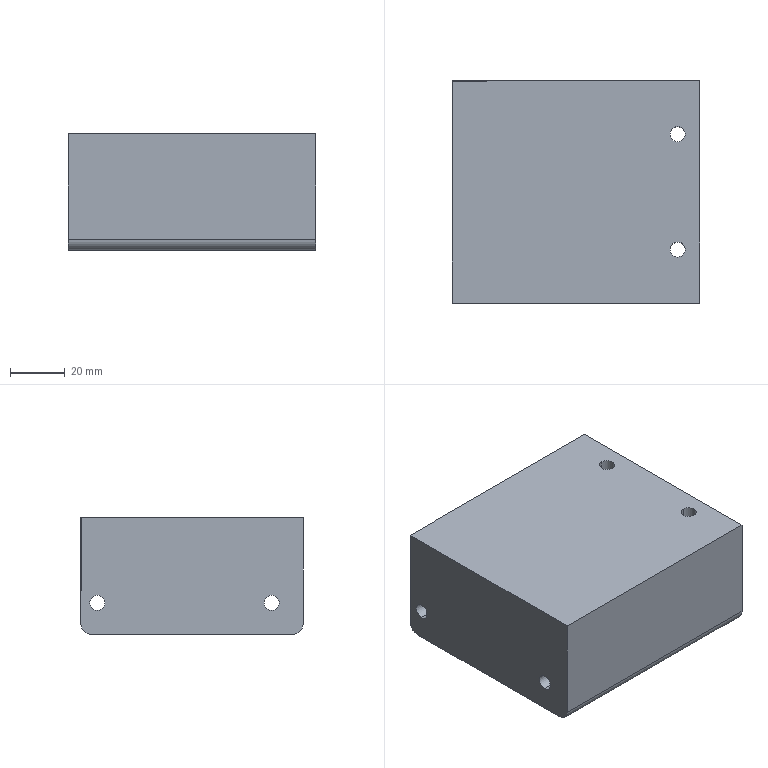Part | STEP file | 复件 FFH80-GY-003A^复件 FFH85-B3 -02_三轴模组 | 1 solid | 55 faces | box 90 x 81 x 42.5 mm | volume 300723 mm3 | cylinder 31 | plane 14 | cone 10 | commonest cylinder face diameters 4.2 x8 5.5 x8 9 x8 2.5 x2 3 x2 8 x2
STEP:
#1=CARTESIAN_POINT('',(82.,23.75,21.25));
#2=VERTEX_POINT('',#1);
#3=CARTESIAN_POINT('',(82.,18.25,21.25));
#4=VERTEX_POINT('',#3);
#5=CARTESIAN_POINT('',(82.,21.,21.25));
#6=DIRECTION('',(0.,0.,1.));
#7=DIRECTION('',(0.,1.,0.));
#8=AXIS2_PLACEMENT_3D('',#5,#6,#7);
#9=CIRCLE('',#8,2.75);
#10=EDGE_CURVE('',#2,#4,#9,.T.);
#11=ORIENTED_EDGE('',*,*,#10,.T.);
#12=CARTESIAN_POINT('',(82.,18.25,-15.25));
#13=VERTEX_POINT('',#12);
#14=CARTESIAN_POINT('',(82.,18.25,-21.25));
#15=DIRECTION('',(0.,0.,-1.));
#16=VECTOR('',#15,1000.);
#17=LINE('',#14,#16);
#18=EDGE_CURVE('',#4,#13,#17,.T.);
#19=ORIENTED_EDGE('',*,*,#18,.T.);
#20=CARTESIAN_POINT('',(82.,23.75,-15.25));
#21=VERTEX_POINT('',#20);
#22=CARTESIAN_POINT('',(82.,21.,-15.25));
#23=DIRECTION('',(0.,0.,1.));
#24=DIRECTION('',(0.,1.,0.));
#25=AXIS2_PLACEMENT_3D('',#22,#23,#24);
#26=CIRCLE('',#25,2.75);
#27=EDGE_CURVE('',#21,#13,#26,.T.);
#28=ORIENTED_EDGE('',*,*,#27,.F.);
#29=CARTESIAN_POINT('',(82.,23.75,-21.25));
#30=DIRECTION('',(0.,0.,-1.));
#31=VECTOR('',#30,1000.);
#32=LINE('',#29,#31);
#33=EDGE_CURVE('',#2,#21,#32,.T.);
#34=ORIENTED_EDGE('',*,*,#33,.F.);
#35=EDGE_LOOP('',(#11,#19,#28,#34));
#36=FACE_OUTER_BOUND('',#35,.T.);
#37=CARTESIAN_POINT('',(82.,21.,-21.25));
#38=DIRECTION('',(0.,0.,-1.));
#39=DIRECTION('',(0.,1.,0.));
#40=AXIS2_PLACEMENT_3D('',#37,#38,#39);
#41=CYLINDRICAL_SURFACE('',#40,2.75);
#42=ADVANCED_FACE('',(#36),#41,.F.);
#43=CARTESIAN_POINT('',(82.,-18.25,21.25));
#44=VERTEX_POINT('',#43);
#45=CARTESIAN_POINT('',(82.,-23.75,21.25));
#46=VERTEX_POINT('',#45);
#47=CARTESIAN_POINT('',(82.,-21.,21.25));
#48=DIRECTION('',(0.,0.,1.));
#49=DIRECTION('',(0.,1.,0.));
#50=AXIS2_PLACEMENT_3D('',#47,#48,#49);
#51=CIRCLE('',#50,2.75);
#52=EDGE_CURVE('',#44,#46,#51,.T.);
#53=ORIENTED_EDGE('',*,*,#52,.T.);
#54=CARTESIAN_POINT('',(82.,-23.75,-15.25));
#55=VERTEX_POINT('',#54);
#56=CARTESIAN_POINT('',(82.,-23.75,-21.25));
#57=DIRECTION('',(0.,0.,-1.));
#58=VECTOR('',#57,1000.);
#59=LINE('',#56,#58);
#60=EDGE_CURVE('',#46,#55,#59,.T.);
#61=ORIENTED_EDGE('',*,*,#60,.T.);
#62=CARTESIAN_POINT('',(82.,-18.25,-15.25));
#63=VERTEX_POINT('',#62);
#64=CARTESIAN_POINT('',(82.,-21.,-15.25));
#65=DIRECTION('',(0.,0.,1.));
#66=DIRECTION('',(0.,1.,0.));
#67=AXIS2_PLACEMENT_3D('',#64,#65,#66);
#68=CIRCLE('',#67,2.75);
#69=EDGE_CURVE('',#63,#55,#68,.T.);
#70=ORIENTED_EDGE('',*,*,#69,.F.);
#71=CARTESIAN_POINT('',(82.,-18.25,-21.25));
#72=DIRECTION('',(0.,0.,-1.));
#73=VECTOR('',#72,1000.);
#74=LINE('',#71,#73);
#75=EDGE_CURVE('',#44,#63,#74,.T.);
#76=ORIENTED_EDGE('',*,*,#75,.F.);
#77=EDGE_LOOP('',(#53,#61,#70,#76));
#78=FACE_OUTER_BOUND('',#77,.T.);
#79=CARTESIAN_POINT('',(82.,-21.,-21.25));
#80=DIRECTION('',(0.,0.,-1.));
#81=DIRECTION('',(0.,1.,0.));
#82=AXIS2_PLACEMENT_3D('',#79,#80,#81);
#83=CYLINDRICAL_SURFACE('',#82,2.75);
#84=ADVANCED_FACE('',(#78),#83,.F.);
#85=CARTESIAN_POINT('',(6.,34.2,3.75));
#86=VERTEX_POINT('',#85);
#87=CARTESIAN_POINT('',(6.,34.2,6.75));
#88=VERTEX_POINT('',#87);
#89=CARTESIAN_POINT('',(6.,34.2,5.25));
#90=DIRECTION('',(0.,1.,0.));
#91=DIRECTION('',(0.,0.,1.));
#92=AXIS2_PLACEMENT_3D('',#89,#90,#91);
#93=CIRCLE('',#92,1.5);
#94=EDGE_CURVE('',#86,#88,#93,.T.);
#95=ORIENTED_EDGE('',*,*,#94,.F.);
#96=CARTESIAN_POINT('',(6.,40.2,3.75));
#97=VERTEX_POINT('',#96);
#98=CARTESIAN_POINT('',(6.,40.2,3.75));
#99=DIRECTION('',(0.,1.,0.));
#100=VECTOR('',#99,1000.);
#101=LINE('',#98,#100);
#102=EDGE_CURVE('',#86,#97,#101,.T.);
#103=ORIENTED_EDGE('',*,*,#102,.T.);
#104=CARTESIAN_POINT('',(6.,40.2,6.75));
#105=VERTEX_POINT('',#104);
#106=CARTESIAN_POINT('',(6.,40.2,5.25));
#107=DIRECTION('',(0.,1.,0.));
#108=DIRECTION('',(0.,0.,1.));
#109=AXIS2_PLACEMENT_3D('',#106,#107,#108);
#110=CIRCLE('',#109,1.5);
#111=EDGE_CURVE('',#97,#105,#110,.T.);
#112=ORIENTED_EDGE('',*,*,#111,.T.);
#113=CARTESIAN_POINT('',(6.,40.2,6.75));
#114=DIRECTION('',(0.,1.,0.));
#115=VECTOR('',#114,1000.);
#116=LINE('',#113,#115);
#117=EDGE_CURVE('',#88,#105,#116,.T.);
#118=ORIENTED_EDGE('',*,*,#117,.F.);
#119=EDGE_LOOP('',(#95,#103,#112,#118));
#120=FACE_OUTER_BOUND('',#119,.T.);
#121=CARTESIAN_POINT('',(6.,40.2,5.25));
#122=DIRECTION('',(0.,1.,0.));
#123=DIRECTION('',(0.,0.,1.));
#124=AXIS2_PLACEMENT_3D('',#121,#122,#123);
#125=CYLINDRICAL_SURFACE('',#124,1.5);
#126=ADVANCED_FACE('',(#120),#125,.F.);
#127=CARTESIAN_POINT('',(0.,34.5,-7.));
#128=VERTEX_POINT('',#127);
#129=CARTESIAN_POINT('',(0.,34.5,-12.5));
#130=VERTEX_POINT('',#129);
#131=CARTESIAN_POINT('',(0.,34.5,-9.75));
#132=DIRECTION('',(1.,0.,0.));
#133=DIRECTION('',(0.,0.,-1.));
#134=AXIS2_PLACEMENT_3D('',#131,#132,#133);
#135=CIRCLE('',#134,2.75);
#136=EDGE_CURVE('',#128,#130,#135,.T.);
#137=ORIENTED_EDGE('',*,*,#136,.F.);
#138=CARTESIAN_POINT('',(84.,34.5,-7.));
#139=VERTEX_POINT('',#138);
#140=CARTESIAN_POINT('',(90.,34.5,-7.));
#141=DIRECTION('',(1.,0.,0.));
#142=VECTOR('',#141,1000.);
#143=LINE('',#140,#142);
#144=EDGE_CURVE('',#128,#139,#143,.T.);
#145=ORIENTED_EDGE('',*,*,#144,.T.);
#146=CARTESIAN_POINT('',(84.,34.5,-12.5));
#147=VERTEX_POINT('',#146);
#148=CARTESIAN_POINT('',(84.,34.5,-9.75));
#149=DIRECTION('',(-1.,0.,0.));
#150=DIRECTION('',(0.,0.,-1.));
#151=AXIS2_PLACEMENT_3D('',#148,#149,#150);
#152=CIRCLE('',#151,2.75);
#153=EDGE_CURVE('',#147,#139,#152,.T.);
#154=ORIENTED_EDGE('',*,*,#153,.F.);
#155=CARTESIAN_POINT('',(90.,34.5,-12.5));
#156=DIRECTION('',(1.,0.,0.));
#157=VECTOR('',#156,1000.);
#158=LINE('',#155,#157);
#159=EDGE_CURVE('',#130,#147,#158,.T.);
#160=ORIENTED_EDGE('',*,*,#159,.F.);
#161=EDGE_LOOP('',(#137,#145,#154,#160));
#162=FACE_OUTER_BOUND('',#161,.T.);
#163=CARTESIAN_POINT('',(90.,34.5,-9.75));
#164=DIRECTION('',(1.,0.,0.));
#165=DIRECTION('',(0.,0.,-1.));
#166=AXIS2_PLACEMENT_3D('',#163,#164,#165);
#167=CYLINDRICAL_SURFACE('',#166,2.75);
#168=ADVANCED_FACE('',(#162),#167,.F.);
#169=CARTESIAN_POINT('',(0.,-29.,-7.));
#170=VERTEX_POINT('',#169);
#171=CARTESIAN_POINT('',(0.,-29.,-12.5));
#172=VERTEX_POINT('',#171);
#173=CARTESIAN_POINT('',(0.,-29.,-9.75));
#174=DIRECTION('',(1.,0.,0.));
#175=DIRECTION('',(0.,0.,-1.));
#176=AXIS2_PLACEMENT_3D('',#173,#174,#175);
#177=CIRCLE('',#176,2.75);
#178=EDGE_CURVE('',#170,#172,#177,.T.);
#179=ORIENTED_EDGE('',*,*,#178,.F.);
#180=CARTESIAN_POINT('',(84.,-29.,-7.));
#181=VERTEX_POINT('',#180);
#182=CARTESIAN_POINT('',(90.,-29.,-7.));
#183=DIRECTION('',(1.,0.,0.));
#184=VECTOR('',#183,1000.);
#185=LINE('',#182,#184);
#186=EDGE_CURVE('',#170,#181,#185,.T.);
#187=ORIENTED_EDGE('',*,*,#186,.T.);
#188=CARTESIAN_POINT('',(84.,-29.,-12.5));
#189=VERTEX_POINT('',#188);
#190=CARTESIAN_POINT('',(84.,-29.,-9.75));
#191=DIRECTION('',(-1.,0.,0.));
#192=DIRECTION('',(0.,0.,-1.));
#193=AXIS2_PLACEMENT_3D('',#190,#191,#192);
#194=CIRCLE('',#193,2.75);
#195=EDGE_CURVE('',#189,#181,#194,.T.);
#196=ORIENTED_EDGE('',*,*,#195,.F.);
#197=CARTESIAN_POINT('',(90.,-29.,-12.5));
#198=DIRECTION('',(1.,0.,0.));
#199=VECTOR('',#198,1000.);
#200=LINE('',#197,#199);
#201=EDGE_CURVE('',#172,#189,#200,.T.);
#202=ORIENTED_EDGE('',*,*,#201,.F.);
#203=EDGE_LOOP('',(#179,#187,#196,#202));
#204=FACE_OUTER_BOUND('',#203,.T.);
#205=CARTESIAN_POINT('',(90.,-29.,-9.75));
#206=DIRECTION('',(1.,0.,0.));
#207=DIRECTION('',(0.,0.,-1.));
#208=AXIS2_PLACEMENT_3D('',#205,#206,#207);
#209=CYLINDRICAL_SURFACE('',#208,2.75);
#210=ADVANCED_FACE('',(#204),#209,.F.);
#211=CARTESIAN_POINT('',(84.,34.5,-5.25));
#212=VERTEX_POINT('',#211);
#213=CARTESIAN_POINT('',(84.,34.5,-14.25));
#214=VERTEX_POINT('',#213);
#215=CARTESIAN_POINT('',(84.,34.5,-9.75));
#216=DIRECTION('',(1.,0.,0.));
#217=DIRECTION('',(0.,0.,-1.));
#218=AXIS2_PLACEMENT_3D('',#215,#216,#217);
#219=CIRCLE('',#218,4.5);
#220=EDGE_CURVE('',#212,#214,#219,.T.);
#221=ORIENTED_EDGE('',*,*,#220,.F.);
#222=CARTESIAN_POINT('',(90.,34.5,-5.25));
#223=VERTEX_POINT('',#222);
#224=CARTESIAN_POINT('',(90.,34.5,-5.25));
#225=DIRECTION('',(1.,0.,0.));
#226=VECTOR('',#225,1000.);
#227=LINE('',#224,#226);
#228=EDGE_CURVE('',#212,#223,#227,.T.);
#229=ORIENTED_EDGE('',*,*,#228,.T.);
#230=CARTESIAN_POINT('',(90.,34.5,-14.25));
#231=VERTEX_POINT('',#230);
#232=CARTESIAN_POINT('',(90.,34.5,-9.75));
#233=DIRECTION('',(1.,0.,0.));
#234=DIRECTION('',(0.,0.,-1.));
#235=AXIS2_PLACEMENT_3D('',#232,#233,#234);
#236=CIRCLE('',#235,4.5);
#237=EDGE_CURVE('',#223,#231,#236,.T.);
#238=ORIENTED_EDGE('',*,*,#237,.T.);
#239=CARTESIAN_POINT('',(90.,34.5,-14.25));
#240=DIRECTION('',(1.,0.,0.));
#241=VECTOR('',#240,1000.);
#242=LINE('',#239,#241);
#243=EDGE_CURVE('',#214,#231,#242,.T.);
#244=ORIENTED_EDGE('',*,*,#243,.F.);
#245=EDGE_LOOP('',(#221,#229,#238,#244));
#246=FACE_OUTER_BOUND('',#245,.T.);
#247=CARTESIAN_POINT('',(90.,34.5,-9.75));
#248=DIRECTION('',(1.,0.,0.));
#249=DIRECTION('',(0.,0.,-1.));
#250=AXIS2_PLACEMENT_3D('',#247,#248,#249);
#251=CYLINDRICAL_SURFACE('',#250,4.5);
#252=ADVANCED_FACE('',(#246),#251,.F.);
#253=CARTESIAN_POINT('',(84.,-29.,-5.25));
#254=VERTEX_POINT('',#253);
#255=CARTESIAN_POINT('',(84.,-29.,-14.25));
#256=VERTEX_POINT('',#255);
#257=CARTESIAN_POINT('',(84.,-29.,-9.75));
#258=DIRECTION('',(1.,0.,0.));
#259=DIRECTION('',(0.,0.,-1.));
#260=AXIS2_PLACEMENT_3D('',#257,#258,#259);
#261=CIRCLE('',#260,4.5);
#262=EDGE_CURVE('',#254,#256,#261,.T.);
#263=ORIENTED_EDGE('',*,*,#262,.F.);
#264=CARTESIAN_POINT('',(90.,-29.,-5.25));
#265=VERTEX_POINT('',#264);
#266=CARTESIAN_POINT('',(90.,-29.,-5.25));
#267=DIRECTION('',(1.,0.,0.));
#268=VECTOR('',#267,1000.);
#269=LINE('',#266,#268);
#270=EDGE_CURVE('',#254,#265,#269,.T.);
#271=ORIENTED_EDGE('',*,*,#270,.T.);
#272=CARTESIAN_POINT('',(90.,-29.,-14.25));
#273=VERTEX_POINT('',#272);
#274=CARTESIAN_POINT('',(90.,-29.,-9.75));
#275=DIRECTION('',(1.,0.,0.));
#276=DIRECTION('',(0.,0.,-1.));
#277=AXIS2_PLACEMENT_3D('',#274,#275,#276);
#278=CIRCLE('',#277,4.5);
#279=EDGE_CURVE('',#265,#273,#278,.T.);
#280=ORIENTED_EDGE('',*,*,#279,.T.);
#281=CARTESIAN_POINT('',(90.,-29.,-14.25));
#282=DIRECTION('',(1.,0.,0.));
#283=VECTOR('',#282,1000.);
#284=LINE('',#281,#283);
#285=EDGE_CURVE('',#256,#273,#284,.T.);
#286=ORIENTED_EDGE('',*,*,#285,.F.);
#287=EDGE_LOOP('',(#263,#271,#280,#286));
#288=FACE_OUTER_BOUND('',#287,.T.);
#289=CARTESIAN_POINT('',(90.,-29.,-9.75));
#290=DIRECTION('',(1.,0.,0.));
#291=DIRECTION('',(0.,0.,-1.));
#292=AXIS2_PLACEMENT_3D('',#289,#290,#291);
#293=CYLINDRICAL_SURFACE('',#292,4.5);
#294=ADVANCED_FACE('',(#288),#293,.F.);
#295=CARTESIAN_POINT('',(82.,25.5,-15.25));
#296=VERTEX_POINT('',#295);
#297=CARTESIAN_POINT('',(82.,16.5,-15.25));
#298=VERTEX_POINT('',#297);
#299=CARTESIAN_POINT('',(82.,21.,-15.25));
#300=DIRECTION('',(0.,0.,1.));
#301=DIRECTION('',(0.,1.,0.));
#302=AXIS2_PLACEMENT_3D('',#299,#300,#301);
#303=CIRCLE('',#302,4.5);
#304=EDGE_CURVE('',#296,#298,#303,.T.);
#305=ORIENTED_EDGE('',*,*,#304,.T.);
#306=CARTESIAN_POINT('',(82.,16.5,-21.25));
#307=VERTEX_POINT('',#306);
#308=CARTESIAN_POINT('',(82.,16.5,-21.25));
#309=DIRECTION('',(0.,0.,-1.));
#310=VECTOR('',#309,1000.);
#311=LINE('',#308,#310);
#312=EDGE_CURVE('',#298,#307,#311,.T.);
#313=ORIENTED_EDGE('',*,*,#312,.T.);
#314=CARTESIAN_POINT('',(82.,25.5,-21.25));
#315=VERTEX_POINT('',#314);
#316=CARTESIAN_POINT('',(82.,21.,-21.25));
#317=DIRECTION('',(0.,0.,-1.));
#318=DIRECTION('',(0.,1.,0.));
#319=AXIS2_PLACEMENT_3D('',#316,#317,#318);
#320=CIRCLE('',#319,4.5);
#321=EDGE_CURVE('',#307,#315,#320,.T.);
#322=ORIENTED_EDGE('',*,*,#321,.T.);
#323=CARTESIAN_POINT('',(82.,25.5,-21.25));
#324=DIRECTION('',(0.,0.,-1.));
#325=VECTOR('',#324,1000.);
#326=LINE('',#323,#325);
#327=EDGE_CURVE('',#296,#315,#326,.T.);
#328=ORIENTED_EDGE('',*,*,#327,.F.);
#329=EDGE_LOOP('',(#305,#313,#322,#328));
#330=FACE_OUTER_BOUND('',#329,.T.);
#331=CARTESIAN_POINT('',(82.,21.,-21.25));
#332=DIRECTION('',(0.,0.,-1.));
#333=DIRECTION('',(0.,1.,0.));
#334=AXIS2_PLACEMENT_3D('',#331,#332,#333);
#335=CYLINDRICAL_SURFACE('',#334,4.5);
#336=ADVANCED_FACE('',(#330),#335,.F.);
#337=CARTESIAN_POINT('',(82.,-16.5,-15.25));
#338=VERTEX_POINT('',#337);
#339=CARTESIAN_POINT('',(82.,-25.5,-15.25));
#340=VERTEX_POINT('',#339);
#341=CARTESIAN_POINT('',(82.,-21.,-15.25));
#342=DIRECTION('',(0.,0.,1.));
#343=DIRECTION('',(0.,1.,0.));
#344=AXIS2_PLACEMENT_3D('',#341,#342,#343);
#345=CIRCLE('',#344,4.5);
#346=EDGE_CURVE('',#338,#340,#345,.T.);
#347=ORIENTED_EDGE('',*,*,#346,.T.);
#348=CARTESIAN_POINT('',(82.,-25.5,-21.25));
#349=VERTEX_POINT('',#348);
#350=CARTESIAN_POINT('',(82.,-25.5,-21.25));
#351=DIRECTION('',(0.,0.,-1.));
#352=VECTOR('',#351,1000.);
#353=LINE('',#350,#352);
#354=EDGE_CURVE('',#340,#349,#353,.T.);
#355=ORIENTED_EDGE('',*,*,#354,.T.);
#356=CARTESIAN_POINT('',(82.,-16.5,-21.25));
#357=VERTEX_POINT('',#356);
#358=CARTESIAN_POINT('',(82.,-21.,-21.25));
#359=DIRECTION('',(0.,0.,-1.));
#360=DIRECTION('',(0.,1.,0.));
#361=AXIS2_PLACEMENT_3D('',#358,#359,#360);
#362=CIRCLE('',#361,4.5);
#363=EDGE_CURVE('',#349,#357,#362,.T.);
#364=ORIENTED_EDGE('',*,*,#363,.T.);
#365=CARTESIAN_POINT('',(82.,-16.5,-21.25));
#366=DIRECTION('',(0.,0.,-1.));
#367=VECTOR('',#366,1000.);
#368=LINE('',#365,#367);
#369=EDGE_CURVE('',#338,#357,#368,.T.);
#370=ORIENTED_EDGE('',*,*,#369,.F.);
#371=EDGE_LOOP('',(#347,#355,#364,#370));
#372=FACE_OUTER_BOUND('',#371,.T.);
#373=CARTESIAN_POINT('',(82.,-21.,-21.25));
#374=DIRECTION('',(0.,0.,-1.));
#375=DIRECTION('',(0.,1.,0.));
#376=AXIS2_PLACEMENT_3D('',#373,#374,#375);
#377=CYLINDRICAL_SURFACE('',#376,4.5);
#378=ADVANCED_FACE('',(#372),#377,.F.);
#379=CARTESIAN_POINT('',(17.5,20.4,-2.25));
#380=VERTEX_POINT('',#379);
#381=CARTESIAN_POINT('',(15.4,22.5,-2.25));
#382=VERTEX_POINT('',#381);
#383=CARTESIAN_POINT('',(17.5,22.5,-2.25));
#384=DIRECTION('',(0.,0.,-1.));
#385=DIRECTION('',(0.,1.,0.));
#386=AXIS2_PLACEMENT_3D('',#383,#384,#385);
#387=CIRCLE('',#386,2.1);
#388=EDGE_CURVE('',#380,#382,#387,.T.);
#389=ORIENTED_EDGE('',*,*,#388,.F.);
#390=CARTESIAN_POINT('',(17.5,20.4,-21.25));
#391=VERTEX_POINT('',#390);
#392=CARTESIAN_POINT('',(17.5,20.4,-21.25));
#393=DIRECTION('',(0.,0.,-1.));
#394=VECTOR('',#393,1000.);
#395=LINE('',#392,#394);
#396=EDGE_CURVE('',#380,#391,#395,.T.);
#397=ORIENTED_EDGE('',*,*,#396,.T.);
#398=CARTESIAN_POINT('',(17.5,24.6,-21.25));
#399=VERTEX_POINT('',#398);
#400=CARTESIAN_POINT('',(17.5,22.5,-21.25));
#401=DIRECTION('',(0.,0.,-1.));
#402=DIRECTION('',(0.,1.,0.));
#403=AXIS2_PLACEMENT_3D('',#400,#401,#402);
#404=CIRCLE('',#403,2.1);
#405=EDGE_CURVE('',#391,#399,#404,.T.);
#406=ORIENTED_EDGE('',*,*,#405,.T.);
#407=CARTESIAN_POINT('',(17.5,24.6,-2.25));
#408=VERTEX_POINT('',#407);
#409=CARTESIAN_POINT('',(17.5,24.6,-21.25));
#410=DIRECTION('',(0.,0.,-1.));
#411=VECTOR('',#410,1000.);
#412=LINE('',#409,#411);
#413=EDGE_CURVE('',#408,#399,#412,.T.);
#414=ORIENTED_EDGE('',*,*,#413,.F.);
#415=CARTESIAN_POINT('',(17.5,22.5,-2.25));
#416=DIRECTION('',(0.,0.,-1.));
#417=DIRECTION('',(0.,1.,0.));
#418=AXIS2_PLACEMENT_3D('',#415,#416,#417);
#419=CIRCLE('',#418,2.1);
#420=EDGE_CURVE('',#382,#408,#419,.T.);
#421=ORIENTED_EDGE('',*,*,#420,.F.);
#422=EDGE_LOOP('',(#389,#397,#406,#414,#421));
#423=FACE_OUTER_BOUND('',#422,.T.);
#424=CARTESIAN_POINT('',(17.5,22.5,-21.25));
#425=DIRECTION('',(0.,0.,-1.));
#426=DIRECTION('',(0.,1.,0.));
#427=AXIS2_PLACEMENT_3D('',#424,#425,#426);
#428=CYLINDRICAL_SURFACE('',#427,2.1);
#429=ADVANCED_FACE('',(#423),#428,.F.);
#430=CARTESIAN_POINT('',(62.5,20.4,-2.25));
#431=VERTEX_POINT('',#430);
#432=CARTESIAN_POINT('',(62.5,24.6,-2.25));
#433=VERTEX_POINT('',#432);
#434=CARTESIAN_POINT('',(62.5,22.5,-2.25));
#435=DIRECTION('',(0.,0.,-1.));
#436=DIRECTION('',(0.,1.,0.));
#437=AXIS2_PLACEMENT_3D('',#434,#435,#436);
#438=CIRCLE('',#437,2.1);
#439=EDGE_CURVE('',#431,#433,#438,.T.);
#440=ORIENTED_EDGE('',*,*,#439,.F.);
#441=CARTESIAN_POINT('',(62.5,20.4,-21.25));
#442=VERTEX_POINT('',#441);
#443=CARTESIAN_POINT('',(62.5,20.4,-21.25));
#444=DIRECTION('',(0.,0.,-1.));
#445=VECTOR('',#444,1000.);
#446=LINE('',#443,#445);
#447=EDGE_CURVE('',#431,#442,#446,.T.);
#448=ORIENTED_EDGE('',*,*,#447,.T.);
#449=CARTESIAN_POINT('',(62.5,24.6,-21.25));
#450=VERTEX_POINT('',#449);
#451=CARTESIAN_POINT('',(62.5,22.5,-21.25));
#452=DIRECTION('',(0.,0.,-1.));
#453=DIRECTION('',(0.,1.,0.));
#454=AXIS2_PLACEMENT_3D('',#451,#452,#453);
#455=CIRCLE('',#454,2.1);
#456=EDGE_CURVE('',#442,#450,#455,.T.);
#457=ORIENTED_EDGE('',*,*,#456,.T.);
#458=CARTESIAN_POINT('',(62.5,24.6,-21.25));
#459=DIRECTION('',(0.,0.,-1.));
#460=VECTOR('',#459,1000.);
#461=LINE('',#458,#460);
#462=EDGE_CURVE('',#433,#450,#461,.T.);
#463=ORIENTED_EDGE('',*,*,#462,.F.);
#464=EDGE_LOOP('',(#440,#448,#457,#463));
#465=FACE_OUTER_BOUND('',#464,.T.);
#466=CARTESIAN_POINT('',(62.5,22.5,-21.25));
#467=DIRECTION('',(0.,0.,-1.));
#468=DIRECTION('',(0.,1.,0.));
#469=AXIS2_PLACEMENT_3D('',#466,#467,#468);
#470=CYLINDRICAL_SURFACE('',#469,2.1);
#471=ADVANCED_FACE('',(#465),#470,.F.);
#472=CARTESIAN_POINT('',(17.5,-24.6,-2.25));
#473=VERTEX_POINT('',#472);
#474=CARTESIAN_POINT('',(17.5,-20.4,-2.25));
#475=VERTEX_POINT('',#474);
#476=CARTESIAN_POINT('',(17.5,-22.5,-2.25));
#477=DIRECTION('',(0.,0.,-1.));
#478=DIRECTION('',(0.,1.,0.));
#479=AXIS2_PLACEMENT_3D('',#476,#477,#478);
#480=CIRCLE('',#479,2.1);
#481=EDGE_CURVE('',#473,#475,#480,.T.);
#482=ORIENTED_EDGE('',*,*,#481,.F.);
#483=CARTESIAN_POINT('',(17.5,-24.6,-21.25));
#484=VERTEX_POINT('',#483);
#485=CARTESIAN_POINT('',(17.5,-24.6,-21.25));
#486=DIRECTION('',(0.,0.,-1.));
#487=VECTOR('',#486,1000.);
#488=LINE('',#485,#487);
#489=EDGE_CURVE('',#473,#484,#488,.T.);
#490=ORIENTED_EDGE('',*,*,#489,.T.);
#491=CARTESIAN_POINT('',(17.5,-20.4,-21.25));
#492=VERTEX_POINT('',#491);
#493=CARTESIAN_POINT('',(17.5,-22.5,-21.25));
#494=DIRECTION('',(0.,0.,-1.));
#495=DIRECTION('',(0.,1.,0.));
#496=AXIS2_PLACEMENT_3D('',#493,#494,#495);
#497=CIRCLE('',#496,2.1);
#498=EDGE_CURVE('',#484,#492,#497,.T.);
#499=ORIENTED_EDGE('',*,*,#498,.T.);
#500=CARTESIAN_POINT('',(17.5,-20.4,-21.25));
#501=DIRECTION('',(0.,0.,-1.));
#502=VECTOR('',#501,1000.);
#503=LINE('',#500,#502);
#504=EDGE_CURVE('',#475,#492,#503,.T.);
#505=ORIENTED_EDGE('',*,*,#504,.F.);
#506=EDGE_LOOP('',(#482,#490,#499,#505));
#507=FACE_OUTER_BOUND('',#506,.T.);
#508=CARTESIAN_POINT('',(17.5,-22.5,-21.25));
#509=DIRECTION('',(0.,0.,-1.));
#510=DIRECTION('',(0.,1.,0.));
#511=AXIS2_PLACEMENT_3D('',#508,#509,#510);
#512=CYLINDRICAL_SURFACE('',#511,2.1);
#513=ADVANCED_FACE('',(#507),#512,.F.);
#514=CARTESIAN_POINT('',(62.5,-24.6,-2.25));
#515=VERTEX_POINT('',#514);
#516=CARTESIAN_POINT('',(62.5,-20.4,-2.25));
#517=VERTEX_POINT('',#516);
#518=CARTESIAN_POINT('',(62.5,-22.5,-2.25));
#519=DIRECTION('',(0.,0.,-1.));
#520=DIRECTION('',(0.,1.,0.));
#521=AXIS2_PLACEMENT_3D('',#518,#519,#520);
#522=CIRCLE('',#521,2.1);
#523=EDGE_CURVE('',#515,#517,#522,.T.);
#524=ORIENTED_EDGE('',*,*,#523,.F.);
#525=CARTESIAN_POINT('',(62.5,-24.6,-21.25));
#526=VERTEX_POINT('',#525);
#527=CARTESIAN_POINT('',(62.5,-24.6,-21.25));
#528=DIRECTION('',(0.,0.,-1.));
#529=VECTOR('',#528,1000.);
#530=LINE('',#527,#529);
#531=EDGE_CURVE('',#515,#526,#530,.T.);
#532=ORIENTED_EDGE('',*,*,#531,.T.);
#533=CARTESIAN_POINT('',(62.5,-20.4,-21.25));
#534=VERTEX_POINT('',#533);
#535=CARTESIAN_POINT('',(62.5,-22.5,-21.25));
#536=DIRECTION('',(0.,0.,-1.));
#537=DIRECTION('',(0.,1.,0.));
#538=AXIS2_PLACEMENT_3D('',#535,#536,#537);
#539=CIRCLE('',#538,2.1);
#540=EDGE_CURVE('',#526,#534,#539,.T.);
#541=ORIENTED_EDGE('',*,*,#540,.T.);
#542=CARTESIAN_POINT('',(62.5,-20.4,-21.25));
#543=DIRECTION('',(0.,0.,-1.));
#544=VECTOR('',#543,1000.);
#545=LINE('',#542,#544);
#546=EDGE_CURVE('',#517,#534,#545,.T.);
#547=ORIENTED_EDGE('',*,*,#546,.F.);
#548=EDGE_LOOP('',(#524,#532,#541,#547));
#549=FACE_OUTER_BOUND('',#548,.T.);
#550=CARTESIAN_POINT('',(62.5,-22.5,-21.25));
#551=DIRECTION('',(0.,0.,-1.));
#552=DIRECTION('',(0.,1.,0.));
#553=AXIS2_PLACEMENT_3D('',#550,#551,#552);
#554=CYLINDRICAL_SURFACE('',#553,2.1);
#555=ADVANCED_FACE('',(#549),#554,.F.);
#556=CARTESIAN_POINT('',(6.,31.7,4.));
#557=VERTEX_POINT('',#556);
#558=CARTESIAN_POINT('',(6.,31.7,6.5));
#559=VERTEX_POINT('',#558);
#560=CARTESIAN_POINT('',(6.,31.7,5.25));
#561=DIRECTION('',(0.,1.,0.));
#562=DIRECTION('',(0.,0.,1.));
#563=AXIS2_PLACEMENT_3D('',#560,#561,#562);
#564=CIRCLE('',#563,1.25);
#565=EDGE_CURVE('',#557,#559,#564,.T.);
#566=ORIENTED_EDGE('',*,*,#565,.F.);
#567=CARTESIAN_POINT('',(6.,34.2,4.));
#568=VERTEX_POINT('',#567);
#569=CARTESIAN_POINT('',(6.,40.2,4.));
#570=DIRECTION('',(0.,1.,0.));
#571=VECTOR('',#570,1000.);
#572=LINE('',#569,#571);
#573=EDGE_CURVE('',#557,#568,#572,.T.);
#574=ORIENTED_EDGE('',*,*,#573,.T.);
#575=CARTESIAN_POINT('',(6.,34.2,6.5));
#576=VERTEX_POINT('',#575);
#577=CARTESIAN_POINT('',(6.,34.2,5.25));
#578=DIRECTION('',(0.,1.,0.));
#579=DIRECTION('',(0.,0.,1.));
#580=AXIS2_PLACEMENT_3D('',#577,#578,#579);
#581=CIRCLE('',#580,1.25);
#582=EDGE_CURVE('',#568,#576,#581,.T.);
#583=ORIENTED_EDGE('',*,*,#582,.T.);
#584=CARTESIAN_POINT('',(6.,40.2,6.5));
#585=DIRECTION('',(0.,1.,0.));
#586=VECTOR('',#585,1000.);
#587=LINE('',#584,#586);
#588=EDGE_CURVE('',#559,#576,#587,.T.);
#589=ORIENTED_EDGE('',*,*,#588,.F.);
#590=EDGE_LOOP('',(#566,#574,#583,#589));
#591=FACE_OUTER_BOUND('',#590,.T.);
#592=CARTESIAN_POINT('',(6.,40.2,5.25));
#593=DIRECTION('',(0.,1.,0.));
#594=DIRECTION('',(0.,0.,1.));
#595=AXIS2_PLACEMENT_3D('',#592,#593,#594);
#596=CYLINDRICAL_SURFACE('',#595,1.25);
#597=ADVANCED_FACE('',(#591),#596,.F.);
#598=CARTESIAN_POINT('',(17.5,22.5,-0.9882));
#599=VERTEX_POINT('',#598);
#600=CARTESIAN_POINT('',(15.4,22.5,-2.25));
#601=DIRECTION('',(-0.8572,0.,-0.515));
#602=VECTOR('',#601,1000.);
#603=LINE('',#600,#602);
#604=EDGE_CURVE('',#599,#382,#603,.T.);
#605=ORIENTED_EDGE('',*,*,#604,.F.);
#606=CARTESIAN_POINT('',(19.6,22.5,-2.25));
#607=VERTEX_POINT('',#606);
#608=CARTESIAN_POINT('',(19.6,22.5,-2.25));
#609=DIRECTION('',(0.8572,0.,-0.515));
#610=VECTOR('',#609,1000.);
#611=LINE('',#608,#610);
#612=EDGE_CURVE('',#599,#607,#611,.T.);
#613=ORIENTED_EDGE('',*,*,#612,.T.);
#614=CARTESIAN_POINT('',(17.5,22.5,-2.25));
#615=DIRECTION('',(0.,0.,-1.));
#616=DIRECTION('',(0.,1.,0.));
#617=AXIS2_PLACEMENT_3D('',#614,#615,#616);
#618=CIRCLE('',#617,2.1);
#619=EDGE_CURVE('',#607,#380,#618,.T.);
#620=ORIENTED_EDGE('',*,*,#619,.T.);
#621=ORIENTED_EDGE('',*,*,#388,.T.);
#622=EDGE_LOOP('',(#605,#613,#620,#621));
#623=FACE_OUTER_BOUND('',#622,.T.);
#624=CARTESIAN_POINT('',(17.5,22.5,-2.25));
#625=DIRECTION('',(0.,0.,-1.));
#626=DIRECTION('',(-1.,0.,0.));
#627=AXIS2_PLACEMENT_3D('',#624,#625,#626);
#628=CONICAL_SURFACE('',#627,2.1,1.03);
#629=ADVANCED_FACE('',(#623),#628,.F.);
#630=CARTESIAN_POINT('',(62.5,22.5,-0.9882));
#631=VERTEX_POINT('',#630);
#632=CARTESIAN_POINT('',(62.5,24.6,-2.25));
#633=DIRECTION('',(0.,0.8572,-0.515));
#634=VECTOR('',#633,1000.);
#635=LINE('',#632,#634);
#636=EDGE_CURVE('',#631,#433,#635,.T.);
#637=ORIENTED_EDGE('',*,*,#636,.F.);
#638=CARTESIAN_POINT('',(62.5,20.4,-2.25));
#639=DIRECTION('',(0.,-0.8572,-0.515));
#640=VECTOR('',#639,1000.);
#641=LINE('',#638,#640);
#642=EDGE_CURVE('',#631,#431,#641,.T.);
#643=ORIENTED_EDGE('',*,*,#642,.T.);
#644=ORIENTED_EDGE('',*,*,#439,.T.);
#645=EDGE_LOOP('',(#637,#643,#644));
#646=FACE_OUTER_BOUND('',#645,.T.);
#647=CARTESIAN_POINT('',(62.5,22.5,-2.25));
#648=DIRECTION('',(0.,0.,-1.));
#649=DIRECTION('',(0.,1.,0.));
#650=AXIS2_PLACEMENT_3D('',#647,#648,#649);
#651=CONICAL_SURFACE('',#650,2.1,1.03);
#652=ADVANCED_FACE('',(#646),#651,.F.);
#653=CARTESIAN_POINT('',(17.5,-22.5,-0.9882));
#654=VERTEX_POINT('',#653);
#655=CARTESIAN_POINT('',(17.5,-20.4,-2.25));
#656=DIRECTION('',(0.,0.8572,-0.515));
#657=VECTOR('',#656,1000.);
#658=LINE('',#655,#657);
#659=EDGE_CURVE('',#654,#475,#658,.T.);
#660=ORIENTED_EDGE('',*,*,#659,.F.);
#661=CARTESIAN_POINT('',(17.5,-24.6,-2.25));
#662=DIRECTION('',(0.,-0.8572,-0.515));
#663=VECTOR('',#662,1000.);
#664=LINE('',#661,#663);
#665=EDGE_CURVE('',#654,#473,#664,.T.);
#666=ORIENTED_EDGE('',*,*,#665,.T.);
#667=ORIENTED_EDGE('',*,*,#481,.T.);
#668=EDGE_LOOP('',(#660,#666,#667));
#669=FACE_OUTER_BOUND('',#668,.T.);
#670=CARTESIAN_POINT('',(17.5,-22.5,-2.25));
#671=DIRECTION('',(0.,0.,-1.));
#672=DIRECTION('',(0.,1.,0.));
#673=AXIS2_PLACEMENT_3D('',#670,#671,#672);
#674=CONICAL_SURFACE('',#673,2.1,1.03);
#675=ADVANCED_FACE('',(#669),#674,.F.);
#676=CARTESIAN_POINT('',(62.5,-22.5,-0.9882));
#677=VERTEX_POINT('',#676);
#678=CARTESIAN_POINT('',(62.5,-20.4,-2.25));
#679=DIRECTION('',(0.,0.8572,-0.515));
#680=VECTOR('',#679,1000.);
#681=LINE('',#678,#680);
#682=EDGE_CURVE('',#677,#517,#681,.T.);
#683=ORIENTED_EDGE('',*,*,#682,.F.);
#684=CARTESIAN_POINT('',(62.5,-24.6,-2.25));
#685=DIRECTION('',(0.,-0.8572,-0.515));
#686=VECTOR('',#685,1000.);
#687=LINE('',#684,#686);
#688=EDGE_CURVE('',#677,#515,#687,.T.);
#689=ORIENTED_EDGE('',*,*,#688,.T.);
#690=ORIENTED_EDGE('',*,*,#523,.T.);
#691=EDGE_LOOP('',(#683,#689,#690));
#692=FACE_OUTER_BOUND('',#691,.T.);
#693=CARTESIAN_POINT('',(62.5,-22.5,-2.25));
#694=DIRECTION('',(0.,0.,-1.));
#695=DIRECTION('',(0.,1.,0.));
#696=AXIS2_PLACEMENT_3D('',#693,#694,#695);
#697=CONICAL_SURFACE('',#696,2.1,1.03);
#698=ADVANCED_FACE('',(#692),#697,.F.);
#699=CARTESIAN_POINT('',(6.,30.949,5.25));
#700=VERTEX_POINT('',#699);
#701=CARTESIAN_POINT('',(6.,31.7,6.5));
#702=DIRECTION('',(0.,0.515,0.8572));
#703=VECTOR('',#702,1000.);
#704=LINE('',#701,#703);
#705=EDGE_CURVE('',#700,#559,#704,.T.);
#706=ORIENTED_EDGE('',*,*,#705,.F.);
#707=CARTESIAN_POINT('',(6.,31.7,4.));
#708=DIRECTION('',(0.,0.515,-0.8572));
#709=VECTOR('',#708,1000.);
#710=LINE('',#707,#709);
#711=EDGE_CURVE('',#700,#557,#710,.T.);
#712=ORIENTED_EDGE('',*,*,#711,.T.);
#713=ORIENTED_EDGE('',*,*,#565,.T.);
#714=EDGE_LOOP('',(#706,#712,#713));
#715=FACE_OUTER_BOUND('',#714,.T.);
#716=CARTESIAN_POINT('',(6.,31.7,5.25));
#717=DIRECTION('',(0.,1.,0.));
#718=DIRECTION('',(0.,0.,1.));
#719=AXIS2_PLACEMENT_3D('',#716,#717,#718);
#720=CONICAL_SURFACE('',#719,1.25,1.03);
#721=ADVANCED_FACE('',(#715),#720,.F.);
#722=ORIENTED_EDGE('',*,*,#10,.F.);
#723=CARTESIAN_POINT('',(82.,21.,21.25));
#724=DIRECTION('',(0.,0.,1.));
#725=DIRECTION('',(0.,1.,0.));
#726=AXIS2_PLACEMENT_3D('',#723,#724,#725);
#727=CIRCLE('',#726,2.75);
#728=EDGE_CURVE('',#4,#2,#727,.T.);
#729=ORIENTED_EDGE('',*,*,#728,.F.);
#730=EDGE_LOOP('',(#722,#729));
#731=FACE_BOUND('',#730,.T.);
#732=ORIENTED_EDGE('',*,*,#52,.F.);
#733=CARTESIAN_POINT('',(82.,-21.,21.25));
#734=DIRECTION('',(0.,0.,1.));
#735=DIRECTION('',(0.,1.,0.));
#736=AXIS2_PLACEMENT_3D('',#733,#734,#735);
#737=CIRCLE('',#736,2.75);
#738=EDGE_CURVE('',#46,#44,#737,.T.);
#739=ORIENTED_EDGE('',*,*,#738,.F.);
#740=EDGE_LOOP('',(#732,#739));
#741=FACE_BOUND('',#740,.T.);
#742=CARTESIAN_POINT('',(0.,40.2,21.25));
#743=VERTEX_POINT('',#742);
#744=CARTESIAN_POINT('',(12.5,40.2,21.25));
#745=VERTEX_POINT('',#744);
#746=CARTESIAN_POINT('',(90.,40.2,21.25));
#747=DIRECTION('',(1.,0.,0.));
#748=VECTOR('',#747,1000.);
#749=LINE('',#746,#748);
#750=EDGE_CURVE('',#743,#745,#749,.T.);
#751=ORIENTED_EDGE('',*,*,#750,.F.);
#752=CARTESIAN_POINT('',(0.,-40.5,21.25));
#753=VERTEX_POINT('',#752);
#754=CARTESIAN_POINT('',(0.,40.5,21.25));
#755=DIRECTION('',(0.,1.,0.));
#756=VECTOR('',#755,1000.);
#757=LINE('',#754,#756);
#758=EDGE_CURVE('',#753,#743,#757,.T.);
#759=ORIENTED_EDGE('',*,*,#758,.F.);
#760=CARTESIAN_POINT('',(90.,-40.5,21.25));
#761=VERTEX_POINT('',#760);
#762=CARTESIAN_POINT('',(90.,-40.5,21.25));
#763=DIRECTION('',(-1.,0.,0.));
#764=VECTOR('',#763,1000.);
#765=LINE('',#762,#764);
#766=EDGE_CURVE('',#761,#753,#765,.T.);
#767=ORIENTED_EDGE('',*,*,#766,.F.);
#768=CARTESIAN_POINT('',(90.,40.5,21.25));
#769=VERTEX_POINT('',#768);
#770=CARTESIAN_POINT('',(90.,40.5,21.25));
#771=DIRECTION('',(0.,-1.,0.));
#772=VECTOR('',#771,1000.);
#773=LINE('',#770,#772);
#774=EDGE_CURVE('',#769,#761,#773,.T.);
#775=ORIENTED_EDGE('',*,*,#774,.F.);
#776=CARTESIAN_POINT('',(12.5,40.5,21.25));
#777=VERTEX_POINT('',#776);
#778=CARTESIAN_POINT('',(90.,40.5,21.25));
#779=DIRECTION('',(1.,0.,0.));
#780=VECTOR('',#779,1000.);
#781=LINE('',#778,#780);
#782=EDGE_CURVE('',#777,#769,#781,.T.);
#783=ORIENTED_EDGE('',*,*,#782,.F.);
#784=CARTESIAN_POINT('',(12.5,40.2,21.25));
#785=DIRECTION('',(0.,-1.,0.));
#786=VECTOR('',#785,1000.);
#787=LINE('',#784,#786);
#788=EDGE_CURVE('',#777,#745,#787,.T.);
#789=ORIENTED_EDGE('',*,*,#788,.T.);
#790=EDGE_LOOP('',(#751,#759,#767,#775,#783,#789));
#791=FACE_OUTER_BOUND('',#790,.T.);
#792=CARTESIAN_POINT('',(90.,40.5,21.25));
#793=DIRECTION('',(0.,0.,-1.));
#794=DIRECTION('',(-1.,0.,0.));
#795=AXIS2_PLACEMENT_3D('',#792,#793,#794);
#796=PLANE('',#795);
#797=ADVANCED_FACE('',(#731,#741,#791),#796,.F.);
#798=ORIENTED_EDGE('',*,*,#18,.F.);
#799=ORIENTED_EDGE('',*,*,#728,.T.);
#800=ORIENTED_EDGE('',*,*,#33,.T.);
#801=CARTESIAN_POINT('',(82.,21.,-15.25));
#802=DIRECTION('',(0.,0.,1.));
#803=DIRECTION('',(0.,1.,0.));
#804=AXIS2_PLACEMENT_3D('',#801,#802,#803);
#805=CIRCLE('',#804,2.75);
#806=EDGE_CURVE('',#13,#21,#805,.T.);
#807=ORIENTED_EDGE('',*,*,#806,.F.);
#808=EDGE_LOOP('',(#798,#799,#800,#807));
#809=FACE_OUTER_BOUND('',#808,.T.);
#810=CARTESIAN_POINT('',(82.,21.,-21.25));
#811=DIRECTION('',(0.,0.,-1.));
#812=DIRECTION('',(0.,1.,0.));
#813=AXIS2_PLACEMENT_3D('',#810,#811,#812);
#814=CYLINDRICAL_SURFACE('',#813,2.75);
#815=ADVANCED_FACE('',(#809),#814,.F.);
#816=ORIENTED_EDGE('',*,*,#60,.F.);
#817=ORIENTED_EDGE('',*,*,#738,.T.);
#818=ORIENTED_EDGE('',*,*,#75,.T.);
#819=CARTESIAN_POINT('',(82.,-21.,-15.25));
#820=DIRECTION('',(0.,0.,1.));
#821=DIRECTION('',(0.,1.,0.));
#822=AXIS2_PLACEMENT_3D('',#819,#820,#821);
#823=CIRCLE('',#822,2.75);
#824=EDGE_CURVE('',#55,#63,#823,.T.);
#825=ORIENTED_EDGE('',*,*,#824,.F.);
#826=EDGE_LOOP('',(#816,#817,#818,#825));
#827=FACE_OUTER_BOUND('',#826,.T.);
#828=CARTESIAN_POINT('',(82.,-21.,-21.25));
#829=DIRECTION('',(0.,0.,-1.));
#830=DIRECTION('',(0.,1.,0.));
#831=AXIS2_PLACEMENT_3D('',#828,#829,#830);
#832=CYLINDRICAL_SURFACE('',#831,2.75);
#833=ADVANCED_FACE('',(#827),#832,.F.);
#834=CARTESIAN_POINT('',(6.,40.2,5.25));
#835=DIRECTION('',(0.,1.,0.));
#836=DIRECTION('',(0.,0.,1.));
#837=AXIS2_PLACEMENT_3D('',#834,#835,#836);
#838=CIRCLE('',#837,1.5);
#839=EDGE_CURVE('',#105,#97,#838,.T.);
#840=ORIENTED_EDGE('',*,*,#839,.F.);
#841=ORIENTED_EDGE('',*,*,#111,.F.);
#842=EDGE_LOOP('',(#840,#841));
#843=FACE_BOUND('',#842,.T.);
#844=CARTESIAN_POINT('',(0.,40.2,-5.25));
#845=VERTEX_POINT('',#844);
#846=CARTESIAN_POINT('',(10.5,40.2,-5.25));
#847=VERTEX_POINT('',#846);
#848=CARTESIAN_POINT('',(0.,40.2,-5.25));
#849=DIRECTION('',(1.,0.,0.));
#850=VECTOR('',#849,1000.);
#851=LINE('',#848,#850);
#852=EDGE_CURVE('',#845,#847,#851,.T.);
#853=ORIENTED_EDGE('',*,*,#852,.F.);
#854=CARTESIAN_POINT('',(0.,40.2,0.));
#855=DIRECTION('',(0.,0.,-1.));
#856=VECTOR('',#855,1000.);
#857=LINE('',#854,#856);
#858=EDGE_CURVE('',#743,#845,#857,.T.);
#859=ORIENTED_EDGE('',*,*,#858,.F.);
#860=ORIENTED_EDGE('',*,*,#750,.T.);
#861=CARTESIAN_POINT('',(12.5,40.2,-3.25));
#862=VERTEX_POINT('',#861);
#863=CARTESIAN_POINT('',(12.5,40.2,0.));
#864=DIRECTION('',(0.,0.,1.));
#865=VECTOR('',#864,1000.);
#866=LINE('',#863,#865);
#867=EDGE_CURVE('',#862,#745,#866,.T.);
#868=ORIENTED_EDGE('',*,*,#867,.F.);
#869=CARTESIAN_POINT('',(10.5,40.2,-3.25));
#870=DIRECTION('',(0.,-1.,0.));
#871=DIRECTION('',(0.,0.,-1.));
#872=AXIS2_PLACEMENT_3D('',#869,#870,#871);
#873=CIRCLE('',#872,2.);
#874=EDGE_CURVE('',#847,#862,#873,.T.);
#875=ORIENTED_EDGE('',*,*,#874,.F.);
#876=EDGE_LOOP('',(#853,#859,#860,#868,#875));
#877=FACE_OUTER_BOUND('',#876,.T.);
#878=CARTESIAN_POINT('',(0.,40.2,0.));
#879=DIRECTION('',(0.,-1.,0.));
#880=DIRECTION('',(0.,0.,-1.));
#881=AXIS2_PLACEMENT_3D('',#878,#879,#880);
#882=PLANE('',#881);
#883=ADVANCED_FACE('',(#843,#877),#882,.F.);
#884=ORIENTED_EDGE('',*,*,#858,.T.);
#885=CARTESIAN_POINT('',(0.,40.5,-5.25));
#886=VERTEX_POINT('',#885);
#887=CARTESIAN_POINT('',(0.,0.,-5.25));
#888=DIRECTION('',(0.,1.,0.));
#889=VECTOR('',#888,1000.);
#890=LINE('',#887,#889);
#891=EDGE_CURVE('',#845,#886,#890,.T.);
#892=ORIENTED_EDGE('',*,*,#891,.T.);
#893=CARTESIAN_POINT('',(0.,40.5,-17.25));
#894=VERTEX_POINT('',#893);
#895=CARTESIAN_POINT('',(0.,40.5,0.));
#896=DIRECTION('',(0.,0.,-1.));
#897=VECTOR('',#896,1000.);
#898=LINE('',#895,#897);
#899=EDGE_CURVE('',#886,#894,#898,.T.);
#900=ORIENTED_EDGE('',*,*,#899,.T.);
#901=CARTESIAN_POINT('',(0.,36.5,-21.25));
#902=VERTEX_POINT('',#901);
#903=CARTESIAN_POINT('',(0.,36.5,-17.25));
#904=DIRECTION('',(-1.,0.,0.));
#905=DIRECTION('',(0.,0.,1.));
#906=AXIS2_PLACEMENT_3D('',#903,#904,#905);
#907=CIRCLE('',#906,4.);
#908=EDGE_CURVE('',#894,#902,#907,.T.);
#909=ORIENTED_EDGE('',*,*,#908,.T.);
#910=CARTESIAN_POINT('',(0.,-36.5,-21.25));
#911=VERTEX_POINT('',#910);
#912=CARTESIAN_POINT('',(0.,0.,-21.25));
#913=DIRECTION('',(0.,-1.,0.));
#914=VECTOR('',#913,1000.);
#915=LINE('',#912,#914);
#916=EDGE_CURVE('',#902,#911,#915,.T.);
#917=ORIENTED_EDGE('',*,*,#916,.T.);
#918=CARTESIAN_POINT('',(0.,-40.5,-17.25));
#919=VERTEX_POINT('',#918);
#920=CARTESIAN_POINT('',(0.,-36.5,-17.25));
#921=DIRECTION('',(-1.,0.,0.));
#922=DIRECTION('',(0.,0.,1.));
#923=AXIS2_PLACEMENT_3D('',#920,#921,#922);
#924=CIRCLE('',#923,4.);
#925=EDGE_CURVE('',#911,#919,#924,.T.);
#926=ORIENTED_EDGE('',*,*,#925,.T.);
#927=CARTESIAN_POINT('',(0.,-40.5,0.));
#928=DIRECTION('',(0.,0.,1.));
#929=VECTOR('',#928,1000.);
#930=LINE('',#927,#929);
#931=EDGE_CURVE('',#919,#753,#930,.T.);
#932=ORIENTED_EDGE('',*,*,#931,.T.);
#933=ORIENTED_EDGE('',*,*,#758,.T.);
#934=EDGE_LOOP('',(#884,#892,#900,#909,#917,#926,#932,#933));
#935=FACE_OUTER_BOUND('',#934,.T.);
#936=CARTESIAN_POINT('',(0.,34.5,-9.75));
#937=DIRECTION('',(1.,0.,0.));
#938=DIRECTION('',(0.,0.,-1.));
#939=AXIS2_PLACEMENT_3D('',#936,#937,#938);
#940=CIRCLE('',#939,2.75);
#941=EDGE_CURVE('',#130,#128,#940,.T.);
#942=ORIENTED_EDGE('',*,*,#941,.T.);
#943=ORIENTED_EDGE('',*,*,#136,.T.);
#944=EDGE_LOOP('',(#942,#943));
#945=FACE_BOUND('',#944,.T.);
#946=CARTESIAN_POINT('',(0.,-29.,-9.75));
#947=DIRECTION('',(1.,0.,0.));
#948=DIRECTION('',(0.,0.,-1.));
#949=AXIS2_PLACEMENT_3D('',#946,#947,#948);
#950=CIRCLE('',#949,2.75);
#951=EDGE_CURVE('',#172,#170,#950,.T.);
#952=ORIENTED_EDGE('',*,*,#951,.T.);
#953=ORIENTED_EDGE('',*,*,#178,.T.);
#954=EDGE_LOOP('',(#952,#953));
#955=FACE_BOUND('',#954,.T.);
#956=CARTESIAN_POINT('',(0.,0.,0.));
#957=DIRECTION('',(-1.,0.,0.));
#958=DIRECTION('',(0.,0.,1.));
#959=AXIS2_PLACEMENT_3D('',#956,#957,#958);
#960=PLANE('',#959);
#961=ADVANCED_FACE('',(#935,#945,#955),#960,.T.);
#962=CARTESIAN_POINT('',(90.,-40.5,-17.25));
#963=VERTEX_POINT('',#962);
#964=CARTESIAN_POINT('',(90.,-40.5,-21.25));
#965=DIRECTION('',(0.,0.,-1.));
#966=VECTOR('',#965,1000.);
#967=LINE('',#964,#966);
#968=EDGE_CURVE('',#761,#963,#967,.T.);
#969=ORIENTED_EDGE('',*,*,#968,.F.);
#970=ORIENTED_EDGE('',*,*,#766,.T.);
#971=ORIENTED_EDGE('',*,*,#931,.F.);
#972=CARTESIAN_POINT('',(90.,-40.5,-17.25));
#973=DIRECTION('',(-1.,0.,0.));
#974=VECTOR('',#973,1000.);
#975=LINE('',#972,#974);
#976=EDGE_CURVE('',#963,#919,#975,.T.);
#977=ORIENTED_EDGE('',*,*,#976,.F.);
#978=EDGE_LOOP('',(#969,#970,#971,#977));
#979=FACE_OUTER_BOUND('',#978,.T.);
#980=CARTESIAN_POINT('',(90.,-40.5,-21.25));
#981=DIRECTION('',(0.,1.,0.));
#982=DIRECTION('',(0.,0.,1.));
#983=AXIS2_PLACEMENT_3D('',#980,#981,#982);
#984=PLANE('',#983);
#985=ADVANCED_FACE('',(#979),#984,.F.);
#986=CARTESIAN_POINT('',(90.,34.5,-9.75));
#987=DIRECTION('',(1.,0.,0.));
#988=DIRECTION('',(0.,0.,-1.));
#989=AXIS2_PLACEMENT_3D('',#986,#987,#988);
#990=CIRCLE('',#989,4.5);
#991=EDGE_CURVE('',#231,#223,#990,.T.);
#992=ORIENTED_EDGE('',*,*,#991,.F.);
#993=ORIENTED_EDGE('',*,*,#237,.F.);
#994=EDGE_LOOP('',(#992,#993));
#995=FACE_BOUND('',#994,.T.);
#996=CARTESIAN_POINT('',(90.,-29.,-9.75));
#997=DIRECTION('',(1.,0.,0.));
#998=DIRECTION('',(0.,0.,-1.));
#999=AXIS2_PLACEMENT_3D('',#996,#997,#998);
#1000=CIRCLE('',#999,4.5);
#1001=EDGE_CURVE('',#273,#265,#1000,.T.);
#1002=ORIENTED_EDGE('',*,*,#1001,.F.);
#1003=ORIENTED_EDGE('',*,*,#279,.F.);
#1004=EDGE_LOOP('',(#1002,#1003));
#1005=FACE_BOUND('',#1004,.T.);
#1006=CARTESIAN_POINT('',(90.,36.5,-21.25));
#1007=VERTEX_POINT('',#1006);
#1008=CARTESIAN_POINT('',(90.,-36.5,-21.25));
#1009=VERTEX_POINT('',#1008);
#1010=CARTESIAN_POINT('',(90.,0.,-21.25));
#1011=DIRECTION('',(0.,-1.,0.));
#1012=VECTOR('',#1011,1000.);
#1013=LINE('',#1010,#1012);
#1014=EDGE_CURVE('',#1007,#1009,#1013,.T.);
#1015=ORIENTED_EDGE('',*,*,#1014,.F.);
#1016=CARTESIAN_POINT('',(90.,40.5,-17.25));
#1017=VERTEX_POINT('',#1016);
#1018=CARTESIAN_POINT('',(90.,36.5,-17.25));
#1019=DIRECTION('',(-1.,0.,0.));
#1020=DIRECTION('',(0.,0.,1.));
#1021=AXIS2_PLACEMENT_3D('',#1018,#1019,#1020);
#1022=CIRCLE('',#1021,4.);
#1023=EDGE_CURVE('',#1017,#1007,#1022,.T.);
#1024=ORIENTED_EDGE('',*,*,#1023,.F.);
#1025=CARTESIAN_POINT('',(90.,40.5,0.));
#1026=DIRECTION('',(0.,0.,-1.));
#1027=VECTOR('',#1026,1000.);
#1028=LINE('',#1025,#1027);
#1029=EDGE_CURVE('',#769,#1017,#1028,.T.);
#1030=ORIENTED_EDGE('',*,*,#1029,.F.);
#1031=ORIENTED_EDGE('',*,*,#774,.T.);
#1032=ORIENTED_EDGE('',*,*,#968,.T.);
#1033=CARTESIAN_POINT('',(90.,-36.5,-17.25));
#1034=DIRECTION('',(-1.,0.,0.));
#1035=DIRECTION('',(0.,0.,1.));
#1036=AXIS2_PLACEMENT_3D('',#1033,#1034,#1035);
#1037=CIRCLE('',#1036,4.);
#1038=EDGE_CURVE('',#1009,#963,#1037,.T.);
#1039=ORIENTED_EDGE('',*,*,#1038,.F.);
#1040=EDGE_LOOP('',(#1015,#1024,#1030,#1031,#1032,#1039));
#1041=FACE_OUTER_BOUND('',#1040,.T.);
#1042=CARTESIAN_POINT('',(90.,0.,0.));
#1043=DIRECTION('',(-1.,0.,0.));
#1044=DIRECTION('',(0.,0.,1.));
#1045=AXIS2_PLACEMENT_3D('',#1042,#1043,#1044);
#1046=PLANE('',#1045);
#1047=ADVANCED_FACE('',(#995,#1005,#1041),#1046,.F.);
#1048=ORIENTED_EDGE('',*,*,#899,.F.);
#1049=CARTESIAN_POINT('',(10.5,40.5,-5.25));
#1050=VERTEX_POINT('',#1049);
#1051=CARTESIAN_POINT('',(90.,40.5,-5.25));
#1052=DIRECTION('',(-1.,0.,0.));
#1053=VECTOR('',#1052,1000.);
#1054=LINE('',#1051,#1053);
#1055=EDGE_CURVE('',#1050,#886,#1054,.T.);
#1056=ORIENTED_EDGE('',*,*,#1055,.F.);
#1057=CARTESIAN_POINT('',(12.5,40.5,-3.25));
#1058=VERTEX_POINT('',#1057);
#1059=CARTESIAN_POINT('',(10.5,40.5,-3.25));
#1060=DIRECTION('',(0.,1.,0.));
#1061=DIRECTION('',(0.,0.,-1.));
#1062=AXIS2_PLACEMENT_3D('',#1059,#1060,#1061);
#1063=CIRCLE('',#1062,2.);
#1064=EDGE_CURVE('',#1058,#1050,#1063,.T.);
#1065=ORIENTED_EDGE('',*,*,#1064,.F.);
#1066=CARTESIAN_POINT('',(12.5,40.5,-21.25));
#1067=DIRECTION('',(0.,0.,-1.));
#1068=VECTOR('',#1067,1000.);
#1069=LINE('',#1066,#1068);
#1070=EDGE_CURVE('',#777,#1058,#1069,.T.);
#1071=ORIENTED_EDGE('',*,*,#1070,.F.);
#1072=ORIENTED_EDGE('',*,*,#782,.T.);
#1073=ORIENTED_EDGE('',*,*,#1029,.T.);
#1074=CARTESIAN_POINT('',(90.,40.5,-17.25));
#1075=DIRECTION('',(1.,0.,0.));
#1076=VECTOR('',#1075,1000.);
#1077=LINE('',#1074,#1076);
#1078=EDGE_CURVE('',#894,#1017,#1077,.T.);
#1079=ORIENTED_EDGE('',*,*,#1078,.F.);
#1080=EDGE_LOOP('',(#1048,#1056,#1065,#1071,#1072,#1073,#1079));
#1081=FACE_OUTER_BOUND('',#1080,.T.);
#1082=CARTESIAN_POINT('',(90.,40.5,-21.25));
#1083=DIRECTION('',(0.,-1.,0.));
#1084=DIRECTION('',(0.,0.,-1.));
#1085=AXIS2_PLACEMENT_3D('',#1082,#1083,#1084);
#1086=PLANE('',#1085);
#1087=ADVANCED_FACE('',(#1081),#1086,.F.);
#1088=ORIENTED_EDGE('',*,*,#27,.T.);
#1089=ORIENTED_EDGE('',*,*,#806,.T.);
#1090=EDGE_LOOP('',(#1088,#1089));
#1091=FACE_BOUND('',#1090,.T.);
#1092=ORIENTED_EDGE('',*,*,#304,.F.);
#1093=CARTESIAN_POINT('',(82.,21.,-15.25));
#1094=DIRECTION('',(0.,0.,1.));
#1095=DIRECTION('',(0.,1.,0.));
#1096=AXIS2_PLACEMENT_3D('',#1093,#1094,#1095);
#1097=CIRCLE('',#1096,4.5);
#1098=EDGE_CURVE('',#298,#296,#1097,.T.);
#1099=ORIENTED_EDGE('',*,*,#1098,.F.);
#1100=EDGE_LOOP('',(#1092,#1099));
#1101=FACE_OUTER_BOUND('',#1100,.T.);
#1102=CARTESIAN_POINT('',(84.75,21.,-15.25));
#1103=DIRECTION('',(0.,0.,1.));
#1104=DIRECTION('',(0.,-1.,0.));
#1105=AXIS2_PLACEMENT_3D('',#1102,#1103,#1104);
#1106=PLANE('',#1105);
#1107=ADVANCED_FACE('',(#1091,#1101),#1106,.F.);
#1108=ORIENTED_EDGE('',*,*,#69,.T.);
#1109=ORIENTED_EDGE('',*,*,#824,.T.);
#1110=EDGE_LOOP('',(#1108,#1109));
#1111=FACE_BOUND('',#1110,.T.);
#1112=ORIENTED_EDGE('',*,*,#346,.F.);
#1113=CARTESIAN_POINT('',(82.,-21.,-15.25));
#1114=DIRECTION('',(0.,0.,1.));
#1115=DIRECTION('',(0.,1.,0.));
#1116=AXIS2_PLACEMENT_3D('',#1113,#1114,#1115);
#1117=CIRCLE('',#1116,4.5);
#1118=EDGE_CURVE('',#340,#338,#1117,.T.);
#1119=ORIENTED_EDGE('',*,*,#1118,.F.);
#1120=EDGE_LOOP('',(#1112,#1119));
#1121=FACE_OUTER_BOUND('',#1120,.T.);
#1122=CARTESIAN_POINT('',(84.75,-21.,-15.25));
#1123=DIRECTION('',(0.,0.,1.));
#1124=DIRECTION('',(0.,-1.,0.));
#1125=AXIS2_PLACEMENT_3D('',#1122,#1123,#1124);
#1126=PLANE('',#1125);
#1127=ADVANCED_FACE('',(#1111,#1121),#1126,.F.);
#1128=ORIENTED_EDGE('',*,*,#102,.F.);
#1129=CARTESIAN_POINT('',(6.,34.2,5.25));
#1130=DIRECTION('',(0.,1.,0.));
#1131=DIRECTION('',(0.,0.,1.));
#1132=AXIS2_PLACEMENT_3D('',#1129,#1130,#1131);
#1133=CIRCLE('',#1132,1.5);
#1134=EDGE_CURVE('',#88,#86,#1133,.T.);
#1135=ORIENTED_EDGE('',*,*,#1134,.F.);
#1136=ORIENTED_EDGE('',*,*,#117,.T.);
#1137=ORIENTED_EDGE('',*,*,#839,.T.);
#1138=EDGE_LOOP('',(#1128,#1135,#1136,#1137));
#1139=FACE_OUTER_BOUND('',#1138,.T.);
#1140=CARTESIAN_POINT('',(6.,40.2,5.25));
#1141=DIRECTION('',(0.,1.,0.));
#1142=DIRECTION('',(0.,0.,1.));
#1143=AXIS2_PLACEMENT_3D('',#1140,#1141,#1142);
#1144=CYLINDRICAL_SURFACE('',#1143,1.5);
#1145=ADVANCED_FACE('',(#1139),#1144,.F.);
#1146=ORIENTED_EDGE('',*,*,#1064,.T.);
#1147=CARTESIAN_POINT('',(10.5,40.2,-5.25));
#1148=DIRECTION('',(0.,1.,0.));
#1149=VECTOR('',#1148,1000.);
#1150=LINE('',#1147,#1149);
#1151=EDGE_CURVE('',#847,#1050,#1150,.T.);
#1152=ORIENTED_EDGE('',*,*,#1151,.F.);
#1153=ORIENTED_EDGE('',*,*,#874,.T.);
#1154=CARTESIAN_POINT('',(12.5,40.2,-3.25));
#1155=DIRECTION('',(0.,-1.,0.));
#1156=VECTOR('',#1155,1000.);
#1157=LINE('',#1154,#1156);
#1158=EDGE_CURVE('',#1058,#862,#1157,.T.);
#1159=ORIENTED_EDGE('',*,*,#1158,.F.);
#1160=EDGE_LOOP('',(#1146,#1152,#1153,#1159));
#1161=FACE_OUTER_BOUND('',#1160,.T.);
#1162=CARTESIAN_POINT('',(10.5,40.2,-3.25));
#1163=DIRECTION('',(0.,-1.,0.));
#1164=DIRECTION('',(0.,0.,-1.));
#1165=AXIS2_PLACEMENT_3D('',#1162,#1163,#1164);
#1166=CYLINDRICAL_SURFACE('',#1165,2.);
#1167=ADVANCED_FACE('',(#1161),#1166,.F.);
#1168=ORIENTED_EDGE('',*,*,#1055,.T.);
#1169=ORIENTED_EDGE('',*,*,#891,.F.);
#1170=ORIENTED_EDGE('',*,*,#852,.T.);
#1171=ORIENTED_EDGE('',*,*,#1151,.T.);
#1172=EDGE_LOOP('',(#1168,#1169,#1170,#1171));
#1173=FACE_OUTER_BOUND('',#1172,.T.);
#1174=CARTESIAN_POINT('',(12.5,40.2,-5.25));
#1175=DIRECTION('',(0.,0.,-1.));
#1176=DIRECTION('',(0.,1.,0.));
#1177=AXIS2_PLACEMENT_3D('',#1174,#1175,#1176);
#1178=PLANE('',#1177);
#1179=ADVANCED_FACE('',(#1173),#1178,.F.);
#1180=ORIENTED_EDGE('',*,*,#867,.T.);
#1181=ORIENTED_EDGE('',*,*,#788,.F.);
#1182=ORIENTED_EDGE('',*,*,#1070,.T.);
#1183=ORIENTED_EDGE('',*,*,#1158,.T.);
#1184=EDGE_LOOP('',(#1180,#1181,#1182,#1183));
#1185=FACE_OUTER_BOUND('',#1184,.T.);
#1186=CARTESIAN_POINT('',(12.5,40.2,-5.25));
#1187=DIRECTION('',(1.,0.,0.));
#1188=DIRECTION('',(0.,0.,-1.));
#1189=AXIS2_PLACEMENT_3D('',#1186,#1187,#1188);
#1190=PLANE('',#1189);
#1191=ADVANCED_FACE('',(#1185),#1190,.F.);
#1192=ORIENTED_EDGE('',*,*,#1038,.T.);
#1193=ORIENTED_EDGE('',*,*,#976,.T.);
#1194=ORIENTED_EDGE('',*,*,#925,.F.);
#1195=CARTESIAN_POINT('',(90.,-36.5,-21.25));
#1196=DIRECTION('',(1.,0.,0.));
#1197=VECTOR('',#1196,1000.);
#1198=LINE('',#1195,#1197);
#1199=EDGE_CURVE('',#911,#1009,#1198,.T.);
#1200=ORIENTED_EDGE('',*,*,#1199,.T.);
#1201=EDGE_LOOP('',(#1192,#1193,#1194,#1200));
#1202=FACE_OUTER_BOUND('',#1201,.T.);
#1203=CARTESIAN_POINT('',(90.,-36.5,-17.25));
#1204=DIRECTION('',(-1.,0.,0.));
#1205=DIRECTION('',(0.,0.,1.));
#1206=AXIS2_PLACEMENT_3D('',#1203,#1204,#1205);
#1207=CYLINDRICAL_SURFACE('',#1206,4.);
#1208=ADVANCED_FACE('',(#1202),#1207,.T.);
#1209=CARTESIAN_POINT('',(17.5,22.5,-21.25));
#1210=DIRECTION('',(0.,0.,-1.));
#1211=DIRECTION('',(0.,1.,0.));
#1212=AXIS2_PLACEMENT_3D('',#1209,#1210,#1211);
#1213=CIRCLE('',#1212,2.1);
#1214=EDGE_CURVE('',#399,#391,#1213,.T.);
#1215=ORIENTED_EDGE('',*,*,#1214,.F.);
#1216=ORIENTED_EDGE('',*,*,#405,.F.);
#1217=EDGE_LOOP('',(#1215,#1216));
#1218=FACE_BOUND('',#1217,.T.);
#1219=CARTESIAN_POINT('',(62.5,22.5,-21.25));
#1220=DIRECTION('',(0.,0.,-1.));
#1221=DIRECTION('',(0.,1.,0.));
#1222=AXIS2_PLACEMENT_3D('',#1219,#1220,#1221);
#1223=CIRCLE('',#1222,2.1);
#1224=EDGE_CURVE('',#450,#442,#1223,.T.);
#1225=ORIENTED_EDGE('',*,*,#1224,.F.);
#1226=ORIENTED_EDGE('',*,*,#456,.F.);
#1227=EDGE_LOOP('',(#1225,#1226));
#1228=FACE_BOUND('',#1227,.T.);
#1229=CARTESIAN_POINT('',(17.5,-22.5,-21.25));
#1230=DIRECTION('',(0.,0.,-1.));
#1231=DIRECTION('',(0.,1.,0.));
#1232=AXIS2_PLACEMENT_3D('',#1229,#1230,#1231);
#1233=CIRCLE('',#1232,2.1);
#1234=EDGE_CURVE('',#492,#484,#1233,.T.);
#1235=ORIENTED_EDGE('',*,*,#1234,.F.);
#1236=ORIENTED_EDGE('',*,*,#498,.F.);
#1237=EDGE_LOOP('',(#1235,#1236));
#1238=FACE_BOUND('',#1237,.T.);
#1239=CARTESIAN_POINT('',(62.5,-22.5,-21.25));
#1240=DIRECTION('',(0.,0.,-1.));
#1241=DIRECTION('',(0.,1.,0.));
#1242=AXIS2_PLACEMENT_3D('',#1239,#1240,#1241);
#1243=CIRCLE('',#1242,2.1);
#1244=EDGE_CURVE('',#534,#526,#1243,.T.);
#1245=ORIENTED_EDGE('',*,*,#1244,.F.);
#1246=ORIENTED_EDGE('',*,*,#540,.F.);
#1247=EDGE_LOOP('',(#1245,#1246));
#1248=FACE_BOUND('',#1247,.T.);
#1249=CARTESIAN_POINT('',(82.,21.,-21.25));
#1250=DIRECTION('',(0.,0.,-1.));
#1251=DIRECTION('',(0.,1.,0.));
#1252=AXIS2_PLACEMENT_3D('',#1249,#1250,#1251);
#1253=CIRCLE('',#1252,4.5);
#1254=EDGE_CURVE('',#315,#307,#1253,.T.);
#1255=ORIENTED_EDGE('',*,*,#1254,.F.);
#1256=ORIENTED_EDGE('',*,*,#321,.F.);
#1257=EDGE_LOOP('',(#1255,#1256));
#1258=FACE_BOUND('',#1257,.T.);
#1259=CARTESIAN_POINT('',(82.,-21.,-21.25));
#1260=DIRECTION('',(0.,0.,-1.));
#1261=DIRECTION('',(0.,1.,0.));
#1262=AXIS2_PLACEMENT_3D('',#1259,#1260,#1261);
#1263=CIRCLE('',#1262,4.5);
#1264=EDGE_CURVE('',#357,#349,#1263,.T.);
#1265=ORIENTED_EDGE('',*,*,#1264,.F.);
#1266=ORIENTED_EDGE('',*,*,#363,.F.);
#1267=EDGE_LOOP('',(#1265,#1266));
#1268=FACE_BOUND('',#1267,.T.);
#1269=ORIENTED_EDGE('',*,*,#916,.F.);
#1270=CARTESIAN_POINT('',(90.,36.5,-21.25));
#1271=DIRECTION('',(-1.,0.,0.));
#1272=VECTOR('',#1271,1000.);
#1273=LINE('',#1270,#1272);
#1274=EDGE_CURVE('',#1007,#902,#1273,.T.);
#1275=ORIENTED_EDGE('',*,*,#1274,.F.);
#1276=ORIENTED_EDGE('',*,*,#1014,.T.);
#1277=ORIENTED_EDGE('',*,*,#1199,.F.);
#1278=EDGE_LOOP('',(#1269,#1275,#1276,#1277));
#1279=FACE_OUTER_BOUND('',#1278,.T.);
#1280=CARTESIAN_POINT('',(90.,40.5,-21.25));
#1281=DIRECTION('',(0.,0.,1.));
#1282=DIRECTION('',(0.,-1.,0.));
#1283=AXIS2_PLACEMENT_3D('',#1280,#1281,#1282);
#1284=PLANE('',#1283);
#1285=ADVANCED_FACE('',(#1218,#1228,#1238,#1248,#1258,#1268,#1279),#1284,.F.);
#1286=ORIENTED_EDGE('',*,*,#1023,.T.);
#1287=ORIENTED_EDGE('',*,*,#1274,.T.);
#1288=ORIENTED_EDGE('',*,*,#908,.F.);
#1289=ORIENTED_EDGE('',*,*,#1078,.T.);
#1290=EDGE_LOOP('',(#1286,#1287,#1288,#1289));
#1291=FACE_OUTER_BOUND('',#1290,.T.);
#1292=CARTESIAN_POINT('',(90.,36.5,-17.25));
#1293=DIRECTION('',(-1.,0.,0.));
#1294=DIRECTION('',(0.,0.,1.));
#1295=AXIS2_PLACEMENT_3D('',#1292,#1293,#1294);
#1296=CYLINDRICAL_SURFACE('',#1295,4.);
#1297=ADVANCED_FACE('',(#1291),#1296,.T.);
#1298=ORIENTED_EDGE('',*,*,#144,.F.);
#1299=ORIENTED_EDGE('',*,*,#941,.F.);
#1300=ORIENTED_EDGE('',*,*,#159,.T.);
#1301=CARTESIAN_POINT('',(84.,34.5,-9.75));
#1302=DIRECTION('',(-1.,0.,0.));
#1303=DIRECTION('',(0.,0.,-1.));
#1304=AXIS2_PLACEMENT_3D('',#1301,#1302,#1303);
#1305=CIRCLE('',#1304,2.75);
#1306=EDGE_CURVE('',#139,#147,#1305,.T.);
#1307=ORIENTED_EDGE('',*,*,#1306,.F.);
#1308=EDGE_LOOP('',(#1298,#1299,#1300,#1307));
#1309=FACE_OUTER_BOUND('',#1308,.T.);
#1310=CARTESIAN_POINT('',(90.,34.5,-9.75));
#1311=DIRECTION('',(1.,0.,0.));
#1312=DIRECTION('',(0.,0.,-1.));
#1313=AXIS2_PLACEMENT_3D('',#1310,#1311,#1312);
#1314=CYLINDRICAL_SURFACE('',#1313,2.75);
#1315=ADVANCED_FACE('',(#1309),#1314,.F.);
#1316=ORIENTED_EDGE('',*,*,#186,.F.);
#1317=ORIENTED_EDGE('',*,*,#951,.F.);
#1318=ORIENTED_EDGE('',*,*,#201,.T.);
#1319=CARTESIAN_POINT('',(84.,-29.,-9.75));
#1320=DIRECTION('',(-1.,0.,0.));
#1321=DIRECTION('',(0.,0.,-1.));
#1322=AXIS2_PLACEMENT_3D('',#1319,#1320,#1321);
#1323=CIRCLE('',#1322,2.75);
#1324=EDGE_CURVE('',#181,#189,#1323,.T.);
#1325=ORIENTED_EDGE('',*,*,#1324,.F.);
#1326=EDGE_LOOP('',(#1316,#1317,#1318,#1325));
#1327=FACE_OUTER_BOUND('',#1326,.T.);
#1328=CARTESIAN_POINT('',(90.,-29.,-9.75));
#1329=DIRECTION('',(1.,0.,0.));
#1330=DIRECTION('',(0.,0.,-1.));
#1331=AXIS2_PLACEMENT_3D('',#1328,#1329,#1330);
#1332=CYLINDRICAL_SURFACE('',#1331,2.75);
#1333=ADVANCED_FACE('',(#1327),#1332,.F.);
#1334=ORIENTED_EDGE('',*,*,#228,.F.);
#1335=CARTESIAN_POINT('',(84.,34.5,-9.75));
#1336=DIRECTION('',(1.,0.,0.));
#1337=DIRECTION('',(0.,0.,-1.));
#1338=AXIS2_PLACEMENT_3D('',#1335,#1336,#1337);
#1339=CIRCLE('',#1338,4.5);
#1340=EDGE_CURVE('',#214,#212,#1339,.T.);
#1341=ORIENTED_EDGE('',*,*,#1340,.F.);
#1342=ORIENTED_EDGE('',*,*,#243,.T.);
#1343=ORIENTED_EDGE('',*,*,#991,.T.);
#1344=EDGE_LOOP('',(#1334,#1341,#1342,#1343));
#1345=FACE_OUTER_BOUND('',#1344,.T.);
#1346=CARTESIAN_POINT('',(90.,34.5,-9.75));
#1347=DIRECTION('',(1.,0.,0.));
#1348=DIRECTION('',(0.,0.,-1.));
#1349=AXIS2_PLACEMENT_3D('',#1346,#1347,#1348);
#1350=CYLINDRICAL_SURFACE('',#1349,4.5);
#1351=ADVANCED_FACE('',(#1345),#1350,.F.);
#1352=ORIENTED_EDGE('',*,*,#270,.F.);
#1353=CARTESIAN_POINT('',(84.,-29.,-9.75));
#1354=DIRECTION('',(1.,0.,0.));
#1355=DIRECTION('',(0.,0.,-1.));
#1356=AXIS2_PLACEMENT_3D('',#1353,#1354,#1355);
#1357=CIRCLE('',#1356,4.5);
#1358=EDGE_CURVE('',#256,#254,#1357,.T.);
#1359=ORIENTED_EDGE('',*,*,#1358,.F.);
#1360=ORIENTED_EDGE('',*,*,#285,.T.);
#1361=ORIENTED_EDGE('',*,*,#1001,.T.);
#1362=EDGE_LOOP('',(#1352,#1359,#1360,#1361));
#1363=FACE_OUTER_BOUND('',#1362,.T.);
#1364=CARTESIAN_POINT('',(90.,-29.,-9.75));
#1365=DIRECTION('',(1.,0.,0.));
#1366=DIRECTION('',(0.,0.,-1.));
#1367=AXIS2_PLACEMENT_3D('',#1364,#1365,#1366);
#1368=CYLINDRICAL_SURFACE('',#1367,4.5);
#1369=ADVANCED_FACE('',(#1363),#1368,.F.);
#1370=ORIENTED_EDGE('',*,*,#312,.F.);
#1371=ORIENTED_EDGE('',*,*,#1098,.T.);
#1372=ORIENTED_EDGE('',*,*,#327,.T.);
#1373=ORIENTED_EDGE('',*,*,#1254,.T.);
#1374=EDGE_LOOP('',(#1370,#1371,#1372,#1373));
#1375=FACE_OUTER_BOUND('',#1374,.T.);
#1376=CARTESIAN_POINT('',(82.,21.,-21.25));
#1377=DIRECTION('',(0.,0.,-1.));
#1378=DIRECTION('',(0.,1.,0.));
#1379=AXIS2_PLACEMENT_3D('',#1376,#1377,#1378);
#1380=CYLINDRICAL_SURFACE('',#1379,4.5);
#1381=ADVANCED_FACE('',(#1375),#1380,.F.);
#1382=ORIENTED_EDGE('',*,*,#354,.F.);
#1383=ORIENTED_EDGE('',*,*,#1118,.T.);
#1384=ORIENTED_EDGE('',*,*,#369,.T.);
#1385=ORIENTED_EDGE('',*,*,#1264,.T.);
#1386=EDGE_LOOP('',(#1382,#1383,#1384,#1385));
#1387=FACE_OUTER_BOUND('',#1386,.T.);
#1388=CARTESIAN_POINT('',(82.,-21.,-21.25));
#1389=DIRECTION('',(0.,0.,-1.));
#1390=DIRECTION('',(0.,1.,0.));
#1391=AXIS2_PLACEMENT_3D('',#1388,#1389,#1390);
#1392=CYLINDRICAL_SURFACE('',#1391,4.5);
#1393=ADVANCED_FACE('',(#1387),#1392,.F.);
#1394=CARTESIAN_POINT('',(6.,34.2,5.25));
#1395=DIRECTION('',(0.,1.,0.));
#1396=DIRECTION('',(0.,0.,1.));
#1397=AXIS2_PLACEMENT_3D('',#1394,#1395,#1396);
#1398=CIRCLE('',#1397,1.25);
#1399=EDGE_CURVE('',#576,#568,#1398,.T.);
#1400=ORIENTED_EDGE('',*,*,#1399,.F.);
#1401=ORIENTED_EDGE('',*,*,#582,.F.);
#1402=EDGE_LOOP('',(#1400,#1401));
#1403=FACE_BOUND('',#1402,.T.);
#1404=ORIENTED_EDGE('',*,*,#1134,.T.);
#1405=ORIENTED_EDGE('',*,*,#94,.T.);
#1406=EDGE_LOOP('',(#1404,#1405));
#1407=FACE_OUTER_BOUND('',#1406,.T.);
#1408=CARTESIAN_POINT('',(7.25,34.2,5.25));
#1409=DIRECTION('',(0.,-1.,0.));
#1410=DIRECTION('',(0.,0.,-1.));
#1411=AXIS2_PLACEMENT_3D('',#1408,#1409,#1410);
#1412=PLANE('',#1411);
#1413=ADVANCED_FACE('',(#1403,#1407),#1412,.F.);
#1414=ORIENTED_EDGE('',*,*,#396,.F.);
#1415=ORIENTED_EDGE('',*,*,#619,.F.);
#1416=CARTESIAN_POINT('',(17.5,22.5,-2.25));
#1417=DIRECTION('',(0.,0.,-1.));
#1418=DIRECTION('',(0.,1.,0.));
#1419=AXIS2_PLACEMENT_3D('',#1416,#1417,#1418);
#1420=CIRCLE('',#1419,2.1);
#1421=EDGE_CURVE('',#408,#607,#1420,.T.);
#1422=ORIENTED_EDGE('',*,*,#1421,.F.);
#1423=ORIENTED_EDGE('',*,*,#413,.T.);
#1424=ORIENTED_EDGE('',*,*,#1214,.T.);
#1425=EDGE_LOOP('',(#1414,#1415,#1422,#1423,#1424));
#1426=FACE_OUTER_BOUND('',#1425,.T.);
#1427=CARTESIAN_POINT('',(17.5,22.5,-21.25));
#1428=DIRECTION('',(0.,0.,-1.));
#1429=DIRECTION('',(0.,1.,0.));
#1430=AXIS2_PLACEMENT_3D('',#1427,#1428,#1429);
#1431=CYLINDRICAL_SURFACE('',#1430,2.1);
#1432=ADVANCED_FACE('',(#1426),#1431,.F.);
#1433=ORIENTED_EDGE('',*,*,#447,.F.);
#1434=CARTESIAN_POINT('',(62.5,22.5,-2.25));
#1435=DIRECTION('',(0.,0.,-1.));
#1436=DIRECTION('',(0.,1.,0.));
#1437=AXIS2_PLACEMENT_3D('',#1434,#1435,#1436);
#1438=CIRCLE('',#1437,2.1);
#1439=EDGE_CURVE('',#433,#431,#1438,.T.);
#1440=ORIENTED_EDGE('',*,*,#1439,.F.);
#1441=ORIENTED_EDGE('',*,*,#462,.T.);
#1442=ORIENTED_EDGE('',*,*,#1224,.T.);
#1443=EDGE_LOOP('',(#1433,#1440,#1441,#1442));
#1444=FACE_OUTER_BOUND('',#1443,.T.);
#1445=CARTESIAN_POINT('',(62.5,22.5,-21.25));
#1446=DIRECTION('',(0.,0.,-1.));
#1447=DIRECTION('',(0.,1.,0.));
#1448=AXIS2_PLACEMENT_3D('',#1445,#1446,#1447);
#1449=CYLINDRICAL_SURFACE('',#1448,2.1);
#1450=ADVANCED_FACE('',(#1444),#1449,.F.);
#1451=ORIENTED_EDGE('',*,*,#489,.F.);
#1452=CARTESIAN_POINT('',(17.5,-22.5,-2.25));
#1453=DIRECTION('',(0.,0.,-1.));
#1454=DIRECTION('',(0.,1.,0.));
#1455=AXIS2_PLACEMENT_3D('',#1452,#1453,#1454);
#1456=CIRCLE('',#1455,2.1);
#1457=EDGE_CURVE('',#475,#473,#1456,.T.);
#1458=ORIENTED_EDGE('',*,*,#1457,.F.);
#1459=ORIENTED_EDGE('',*,*,#504,.T.);
#1460=ORIENTED_EDGE('',*,*,#1234,.T.);
#1461=EDGE_LOOP('',(#1451,#1458,#1459,#1460));
#1462=FACE_OUTER_BOUND('',#1461,.T.);
#1463=CARTESIAN_POINT('',(17.5,-22.5,-21.25));
#1464=DIRECTION('',(0.,0.,-1.));
#1465=DIRECTION('',(0.,1.,0.));
#1466=AXIS2_PLACEMENT_3D('',#1463,#1464,#1465);
#1467=CYLINDRICAL_SURFACE('',#1466,2.1);
#1468=ADVANCED_FACE('',(#1462),#1467,.F.);
#1469=ORIENTED_EDGE('',*,*,#531,.F.);
#1470=CARTESIAN_POINT('',(62.5,-22.5,-2.25));
#1471=DIRECTION('',(0.,0.,-1.));
#1472=DIRECTION('',(0.,1.,0.));
#1473=AXIS2_PLACEMENT_3D('',#1470,#1471,#1472);
#1474=CIRCLE('',#1473,2.1);
#1475=EDGE_CURVE('',#517,#515,#1474,.T.);
#1476=ORIENTED_EDGE('',*,*,#1475,.F.);
#1477=ORIENTED_EDGE('',*,*,#546,.T.);
#1478=ORIENTED_EDGE('',*,*,#1244,.T.);
#1479=EDGE_LOOP('',(#1469,#1476,#1477,#1478));
#1480=FACE_OUTER_BOUND('',#1479,.T.);
#1481=CARTESIAN_POINT('',(62.5,-22.5,-21.25));
#1482=DIRECTION('',(0.,0.,-1.));
#1483=DIRECTION('',(0.,1.,0.));
#1484=AXIS2_PLACEMENT_3D('',#1481,#1482,#1483);
#1485=CYLINDRICAL_SURFACE('',#1484,2.1);
#1486=ADVANCED_FACE('',(#1480),#1485,.F.);
#1487=ORIENTED_EDGE('',*,*,#153,.T.);
#1488=ORIENTED_EDGE('',*,*,#1306,.T.);
#1489=EDGE_LOOP('',(#1487,#1488));
#1490=FACE_BOUND('',#1489,.T.);
#1491=ORIENTED_EDGE('',*,*,#1340,.T.);
#1492=ORIENTED_EDGE('',*,*,#220,.T.);
#1493=EDGE_LOOP('',(#1491,#1492));
#1494=FACE_OUTER_BOUND('',#1493,.T.);
#1495=CARTESIAN_POINT('',(84.,37.25,-9.75));
#1496=DIRECTION('',(-1.,0.,0.));
#1497=DIRECTION('',(0.,0.,1.));
#1498=AXIS2_PLACEMENT_3D('',#1495,#1496,#1497);
#1499=PLANE('',#1498);
#1500=ADVANCED_FACE('',(#1490,#1494),#1499,.F.);
#1501=ORIENTED_EDGE('',*,*,#195,.T.);
#1502=ORIENTED_EDGE('',*,*,#1324,.T.);
#1503=EDGE_LOOP('',(#1501,#1502));
#1504=FACE_BOUND('',#1503,.T.);
#1505=ORIENTED_EDGE('',*,*,#1358,.T.);
#1506=ORIENTED_EDGE('',*,*,#262,.T.);
#1507=EDGE_LOOP('',(#1505,#1506));
#1508=FACE_OUTER_BOUND('',#1507,.T.);
#1509=CARTESIAN_POINT('',(84.,-26.25,-9.75));
#1510=DIRECTION('',(-1.,0.,0.));
#1511=DIRECTION('',(0.,0.,1.));
#1512=AXIS2_PLACEMENT_3D('',#1509,#1510,#1511);
#1513=PLANE('',#1512);
#1514=ADVANCED_FACE('',(#1504,#1508),#1513,.F.);
#1515=ORIENTED_EDGE('',*,*,#573,.F.);
#1516=CARTESIAN_POINT('',(6.,31.7,5.25));
#1517=DIRECTION('',(0.,1.,0.));
#1518=DIRECTION('',(0.,0.,1.));
#1519=AXIS2_PLACEMENT_3D('',#1516,#1517,#1518);
#1520=CIRCLE('',#1519,1.25);
#1521=EDGE_CURVE('',#559,#557,#1520,.T.);
#1522=ORIENTED_EDGE('',*,*,#1521,.F.);
#1523=ORIENTED_EDGE('',*,*,#588,.T.);
#1524=ORIENTED_EDGE('',*,*,#1399,.T.);
#1525=EDGE_LOOP('',(#1515,#1522,#1523,#1524));
#1526=FACE_OUTER_BOUND('',#1525,.T.);
#1527=CARTESIAN_POINT('',(6.,40.2,5.25));
#1528=DIRECTION('',(0.,1.,0.));
#1529=DIRECTION('',(0.,0.,1.));
#1530=AXIS2_PLACEMENT_3D('',#1527,#1528,#1529);
#1531=CYLINDRICAL_SURFACE('',#1530,1.25);
#1532=ADVANCED_FACE('',(#1526),#1531,.F.);
#1533=ORIENTED_EDGE('',*,*,#612,.F.);
#1534=ORIENTED_EDGE('',*,*,#604,.T.);
#1535=ORIENTED_EDGE('',*,*,#420,.T.);
#1536=ORIENTED_EDGE('',*,*,#1421,.T.);
#1537=EDGE_LOOP('',(#1533,#1534,#1535,#1536));
#1538=FACE_OUTER_BOUND('',#1537,.T.);
#1539=CARTESIAN_POINT('',(17.5,22.5,-2.25));
#1540=DIRECTION('',(0.,0.,-1.));
#1541=DIRECTION('',(-1.,0.,0.));
#1542=AXIS2_PLACEMENT_3D('',#1539,#1540,#1541);
#1543=CONICAL_SURFACE('',#1542,2.1,1.03);
#1544=ADVANCED_FACE('',(#1538),#1543,.F.);
#1545=ORIENTED_EDGE('',*,*,#642,.F.);
#1546=ORIENTED_EDGE('',*,*,#636,.T.);
#1547=ORIENTED_EDGE('',*,*,#1439,.T.);
#1548=EDGE_LOOP('',(#1545,#1546,#1547));
#1549=FACE_OUTER_BOUND('',#1548,.T.);
#1550=CARTESIAN_POINT('',(62.5,22.5,-2.25));
#1551=DIRECTION('',(0.,0.,-1.));
#1552=DIRECTION('',(0.,1.,0.));
#1553=AXIS2_PLACEMENT_3D('',#1550,#1551,#1552);
#1554=CONICAL_SURFACE('',#1553,2.1,1.03);
#1555=ADVANCED_FACE('',(#1549),#1554,.F.);
#1556=ORIENTED_EDGE('',*,*,#665,.F.);
#1557=ORIENTED_EDGE('',*,*,#659,.T.);
#1558=ORIENTED_EDGE('',*,*,#1457,.T.);
#1559=EDGE_LOOP('',(#1556,#1557,#1558));
#1560=FACE_OUTER_BOUND('',#1559,.T.);
#1561=CARTESIAN_POINT('',(17.5,-22.5,-2.25));
#1562=DIRECTION('',(0.,0.,-1.));
#1563=DIRECTION('',(0.,1.,0.));
#1564=AXIS2_PLACEMENT_3D('',#1561,#1562,#1563);
#1565=CONICAL_SURFACE('',#1564,2.1,1.03);
#1566=ADVANCED_FACE('',(#1560),#1565,.F.);
#1567=ORIENTED_EDGE('',*,*,#688,.F.);
#1568=ORIENTED_EDGE('',*,*,#682,.T.);
#1569=ORIENTED_EDGE('',*,*,#1475,.T.);
#1570=EDGE_LOOP('',(#1567,#1568,#1569));
#1571=FACE_OUTER_BOUND('',#1570,.T.);
#1572=CARTESIAN_POINT('',(62.5,-22.5,-2.25));
#1573=DIRECTION('',(0.,0.,-1.));
#1574=DIRECTION('',(0.,1.,0.));
#1575=AXIS2_PLACEMENT_3D('',#1572,#1573,#1574);
#1576=CONICAL_SURFACE('',#1575,2.1,1.03);
#1577=ADVANCED_FACE('',(#1571),#1576,.F.);
#1578=ORIENTED_EDGE('',*,*,#711,.F.);
#1579=ORIENTED_EDGE('',*,*,#705,.T.);
#1580=ORIENTED_EDGE('',*,*,#1521,.T.);
#1581=EDGE_LOOP('',(#1578,#1579,#1580));
#1582=FACE_OUTER_BOUND('',#1581,.T.);
#1583=CARTESIAN_POINT('',(6.,31.7,5.25));
#1584=DIRECTION('',(0.,1.,0.));
#1585=DIRECTION('',(0.,0.,1.));
#1586=AXIS2_PLACEMENT_3D('',#1583,#1584,#1585);
#1587=CONICAL_SURFACE('',#1586,1.25,1.03);
#1588=ADVANCED_FACE('',(#1582),#1587,.F.);
#1589=CLOSED_SHELL('',(#42,#84,#126,#168,#210,#252,#294,#336,#378,#429,#471,#513,#555,#597,#629,#652,#675,#698,#721,#797,#815,#833,#883,#961,#985,#1047,#1087,#1107,#1127,#1145,#1167,#1179,#1191,#1208,#1285,#1297,#1315,#1333,#1351,#1369,#1381,#1393,#1413,#1432,#1450,#1468,#1486,#1500,#1514,#1532,#1544,#1555,#1566,#1577,#1588));
#1590=MANIFOLD_SOLID_BREP('',#1589);
#1591=CARTESIAN_POINT('',(0.,0.,0.));
#1592=DIRECTION('',(0.,0.,1.));
#1593=DIRECTION('',(1.,0.,0.));
#1594=AXIS2_PLACEMENT_3D('',#1591,#1592,#1593);
#1595=(LENGTH_UNIT()NAMED_UNIT(*)SI_UNIT(.MILLI.,.METRE.));
#1596=UNCERTAINTY_MEASURE_WITH_UNIT(LENGTH_MEASURE(0.00001),#1595,'','');
#1597=(NAMED_UNIT(*)PLANE_ANGLE_UNIT()SI_UNIT($,.RADIAN.));
#1598=(NAMED_UNIT(*)SI_UNIT($,.STERADIAN.)SOLID_ANGLE_UNIT());
#1599=(GEOMETRIC_REPRESENTATION_CONTEXT(3)GLOBAL_UNCERTAINTY_ASSIGNED_CONTEXT((#1596))GLOBAL_UNIT_ASSIGNED_CONTEXT((#1595,#1597,#1598))REPRESENTATION_CONTEXT('',''));
#1600=ADVANCED_BREP_SHAPE_REPRESENTATION('',(#1590,#1594),#1599);